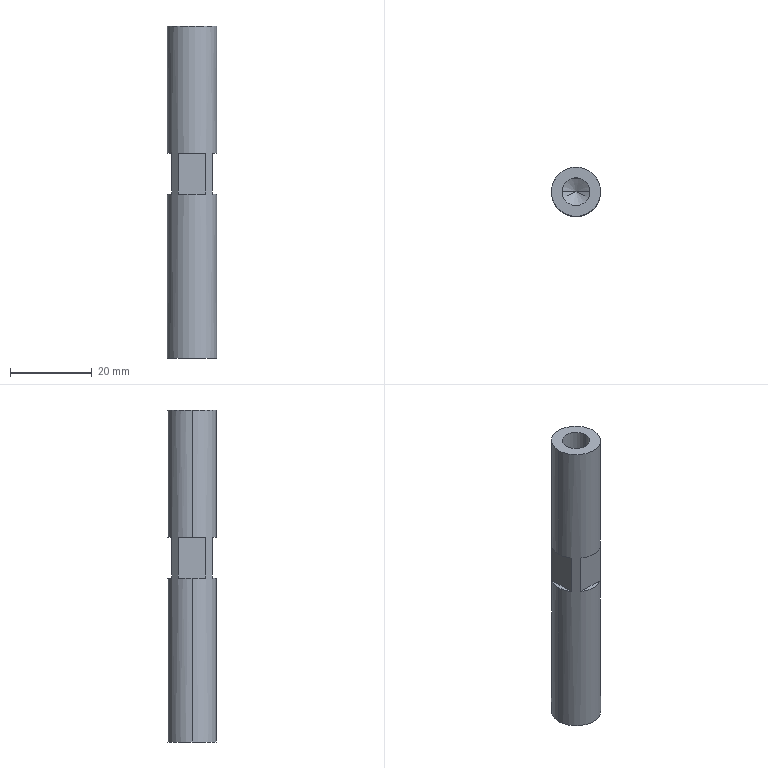Part | STEP file | 44-02-10 Ear Forming Connecting Rod | 1 solid | 24 faces | box 12 x 12 x 81 mm | volume 7569 mm3 | plane 14 | cylinder 6 | cone 4 | commonest cylinder face diameters 6.8 x4 12 x2
STEP:
#1=CARTESIAN_POINT('',(0.,0.,0.));
#2=DIRECTION('',(0.,0.,1.));
#3=DIRECTION('',(1.,0.,0.));
#4=AXIS2_PLACEMENT_3D('',#1,#2,#3);
#5=CARTESIAN_POINT('',(-3.4,0.,-21.75));
#6=VERTEX_POINT('',#5);
#7=CARTESIAN_POINT('',(-3.4,0.,-40.5));
#8=VERTEX_POINT('',#7);
#9=CARTESIAN_POINT('',(-3.4,0.,-40.5));
#10=DIRECTION('',(0.,0.,-1.));
#11=VECTOR('',#10,1.);
#12=LINE('',#9,#11);
#13=CARTESIAN_POINT('',(0.,0.,-40.5));
#14=DIRECTION('',(0.,0.,-1.));
#15=DIRECTION('',(-1.,0.,0.));
#16=AXIS2_PLACEMENT_3D('',#13,#14,#15);
#17=CYLINDRICAL_SURFACE('',#16,3.4);
#18=CARTESIAN_POINT('',(6.283,0.));
#19=DIRECTION('',(0.,1.));
#20=VECTOR('',#19,1.);
#21=LINE('',#18,#20);
#22=(GEOMETRIC_REPRESENTATION_CONTEXT(2)PARAMETRIC_REPRESENTATION_CONTEXT()REPRESENTATION_CONTEXT('',''));
#23=DEFINITIONAL_REPRESENTATION('',(#21),#22);
#24=PCURVE('',#17,#23);
#25=CARTESIAN_POINT('',(0.,0.,-40.5));
#26=DIRECTION('',(0.,0.,-1.));
#27=DIRECTION('',(-1.,0.,0.));
#28=AXIS2_PLACEMENT_3D('',#25,#26,#27);
#29=CYLINDRICAL_SURFACE('',#28,3.4);
#30=CARTESIAN_POINT('',(0.,0.));
#31=DIRECTION('',(0.,1.));
#32=VECTOR('',#31,1.);
#33=LINE('',#30,#32);
#34=(GEOMETRIC_REPRESENTATION_CONTEXT(2)PARAMETRIC_REPRESENTATION_CONTEXT()REPRESENTATION_CONTEXT('',''));
#35=DEFINITIONAL_REPRESENTATION('',(#33),#34);
#36=PCURVE('',#29,#35);
#37=SURFACE_CURVE('',#12,(#24,#36),.PCURVE_S1.);
#38=EDGE_CURVE('',#6,#8,#37,.T.);
#39=ORIENTED_EDGE('',*,*,#38,.T.);
#40=CARTESIAN_POINT('',(3.4,0.,-40.5));
#41=VERTEX_POINT('',#40);
#42=CARTESIAN_POINT('',(0.,0.,-40.5));
#43=DIRECTION('',(0.,0.,-1.));
#44=DIRECTION('',(-1.,0.,0.));
#45=AXIS2_PLACEMENT_3D('',#42,#43,#44);
#46=CIRCLE('',#45,3.4);
#47=CARTESIAN_POINT('',(0.,0.));
#48=DIRECTION('',(1.,0.));
#49=VECTOR('',#48,1.);
#50=LINE('',#47,#49);
#51=(GEOMETRIC_REPRESENTATION_CONTEXT(2)PARAMETRIC_REPRESENTATION_CONTEXT()REPRESENTATION_CONTEXT('',''));
#52=DEFINITIONAL_REPRESENTATION('',(#50),#51);
#53=PCURVE('',#17,#52);
#54=CARTESIAN_POINT('',(0.,0.,-40.5));
#55=DIRECTION('',(0.,0.,1.));
#56=DIRECTION('',(1.,0.,0.));
#57=AXIS2_PLACEMENT_3D('',#54,#55,#56);
#58=PLANE('',#57);
#59=CARTESIAN_POINT('',(-3.4,0.));
#60=CARTESIAN_POINT('',(-3.4,5.889));
#61=CARTESIAN_POINT('',(1.7,2.944));
#62=CARTESIAN_POINT('',(6.8,0.));
#63=CARTESIAN_POINT('',(1.7,-2.944));
#64=CARTESIAN_POINT('',(-3.4,-5.889));
#65=CARTESIAN_POINT('',(-3.4,0.));
#66=(BOUNDED_CURVE()B_SPLINE_CURVE(2,(#59,#60,#61,#62,#63,#64,#65),.UNSPECIFIED.,.T.,.F.)B_SPLINE_CURVE_WITH_KNOTS((1,2,2,2,2,1),(-2.094,0.,2.094,4.189,6.283,8.378),.UNSPECIFIED.)CURVE()GEOMETRIC_REPRESENTATION_ITEM()RATIONAL_B_SPLINE_CURVE((1.,0.5,1.,0.5,1.,0.5,1.))REPRESENTATION_ITEM(''));
#67=(GEOMETRIC_REPRESENTATION_CONTEXT(2)PARAMETRIC_REPRESENTATION_CONTEXT()REPRESENTATION_CONTEXT('',''));
#68=DEFINITIONAL_REPRESENTATION('',(#66),#67);
#69=PCURVE('',#58,#68);
#70=SURFACE_CURVE('',#46,(#53,#69),.PCURVE_S1.);
#71=EDGE_CURVE('',#41,#8,#70,.T.);
#72=ORIENTED_EDGE('',*,*,#71,.F.);
#73=CARTESIAN_POINT('',(3.4,0.,-21.75));
#74=VERTEX_POINT('',#73);
#75=CARTESIAN_POINT('',(3.4,0.,-40.5));
#76=DIRECTION('',(0.,0.,-1.));
#77=VECTOR('',#76,1.);
#78=LINE('',#75,#77);
#79=CARTESIAN_POINT('',(3.142,0.));
#80=DIRECTION('',(0.,1.));
#81=VECTOR('',#80,1.);
#82=LINE('',#79,#81);
#83=(GEOMETRIC_REPRESENTATION_CONTEXT(2)PARAMETRIC_REPRESENTATION_CONTEXT()REPRESENTATION_CONTEXT('',''));
#84=DEFINITIONAL_REPRESENTATION('',(#82),#83);
#85=PCURVE('',#17,#84);
#86=CARTESIAN_POINT('',(3.142,0.));
#87=DIRECTION('',(0.,1.));
#88=VECTOR('',#87,1.);
#89=LINE('',#86,#88);
#90=(GEOMETRIC_REPRESENTATION_CONTEXT(2)PARAMETRIC_REPRESENTATION_CONTEXT()REPRESENTATION_CONTEXT('',''));
#91=DEFINITIONAL_REPRESENTATION('',(#89),#90);
#92=PCURVE('',#29,#91);
#93=SURFACE_CURVE('',#78,(#85,#92),.PCURVE_S1.);
#94=EDGE_CURVE('',#74,#41,#93,.T.);
#95=ORIENTED_EDGE('',*,*,#94,.F.);
#96=CARTESIAN_POINT('',(0.,0.,-21.75));
#97=DIRECTION('',(0.,0.,-1.));
#98=DIRECTION('',(-1.,0.,0.));
#99=AXIS2_PLACEMENT_3D('',#96,#97,#98);
#100=CIRCLE('',#99,3.4);
#101=CARTESIAN_POINT('',(0.,-18.75));
#102=DIRECTION('',(1.,0.));
#103=VECTOR('',#102,1.);
#104=LINE('',#101,#103);
#105=(GEOMETRIC_REPRESENTATION_CONTEXT(2)PARAMETRIC_REPRESENTATION_CONTEXT()REPRESENTATION_CONTEXT('',''));
#106=DEFINITIONAL_REPRESENTATION('',(#104),#105);
#107=PCURVE('',#17,#106);
#108=CARTESIAN_POINT('',(0.,0.,-21.75));
#109=DIRECTION('',(0.,0.,-1.));
#110=DIRECTION('',(-1.,0.,0.));
#111=AXIS2_PLACEMENT_3D('',#108,#109,#110);
#112=CONICAL_SURFACE('',#111,3.4,1.03);
#113=CARTESIAN_POINT('',(0.,0.));
#114=DIRECTION('',(1.,0.));
#115=VECTOR('',#114,1.);
#116=LINE('',#113,#115);
#117=(GEOMETRIC_REPRESENTATION_CONTEXT(2)PARAMETRIC_REPRESENTATION_CONTEXT()REPRESENTATION_CONTEXT('',''));
#118=DEFINITIONAL_REPRESENTATION('',(#116),#117);
#119=PCURVE('',#112,#118);
#120=SURFACE_CURVE('',#100,(#107,#119),.PCURVE_S1.);
#121=EDGE_CURVE('',#74,#6,#120,.T.);
#122=ORIENTED_EDGE('',*,*,#121,.T.);
#123=EDGE_LOOP('',(#39,#72,#95,#122));
#124=FACE_BOUND('',#123,.F.);
#125=ADVANCED_FACE('',(#124),#17,.F.);
#126=ORIENTED_EDGE('',*,*,#121,.F.);
#127=CARTESIAN_POINT('',(0.,0.,-19.707));
#128=VERTEX_POINT('',#127);
#129=CARTESIAN_POINT('',(3.4,0.,-21.75));
#130=DIRECTION('',(0.8572,0.,-0.515));
#131=VECTOR('',#130,1.);
#132=LINE('',#129,#131);
#133=CARTESIAN_POINT('',(3.142,0.));
#134=DIRECTION('',(0.,1.));
#135=VECTOR('',#134,1.);
#136=LINE('',#133,#135);
#137=(GEOMETRIC_REPRESENTATION_CONTEXT(2)PARAMETRIC_REPRESENTATION_CONTEXT()REPRESENTATION_CONTEXT('',''));
#138=DEFINITIONAL_REPRESENTATION('',(#136),#137);
#139=PCURVE('',#112,#138);
#140=CARTESIAN_POINT('',(0.,0.,-21.75));
#141=DIRECTION('',(0.,0.,-1.));
#142=DIRECTION('',(-1.,0.,0.));
#143=AXIS2_PLACEMENT_3D('',#140,#141,#142);
#144=CONICAL_SURFACE('',#143,3.4,1.03);
#145=CARTESIAN_POINT('',(3.142,0.));
#146=DIRECTION('',(0.,1.));
#147=VECTOR('',#146,1.);
#148=LINE('',#145,#147);
#149=(GEOMETRIC_REPRESENTATION_CONTEXT(2)PARAMETRIC_REPRESENTATION_CONTEXT()REPRESENTATION_CONTEXT('',''));
#150=DEFINITIONAL_REPRESENTATION('',(#148),#149);
#151=PCURVE('',#144,#150);
#152=SURFACE_CURVE('',#132,(#139,#151),.PCURVE_S1.);
#153=EDGE_CURVE('',#128,#74,#152,.T.);
#154=ORIENTED_EDGE('',*,*,#153,.F.);
#155=CARTESIAN_POINT('',(-3.4,0.,-21.75));
#156=DIRECTION('',(-0.8572,0.,-0.515));
#157=VECTOR('',#156,1.);
#158=LINE('',#155,#157);
#159=CARTESIAN_POINT('',(6.283,0.));
#160=DIRECTION('',(0.,1.));
#161=VECTOR('',#160,1.);
#162=LINE('',#159,#161);
#163=(GEOMETRIC_REPRESENTATION_CONTEXT(2)PARAMETRIC_REPRESENTATION_CONTEXT()REPRESENTATION_CONTEXT('',''));
#164=DEFINITIONAL_REPRESENTATION('',(#162),#163);
#165=PCURVE('',#112,#164);
#166=CARTESIAN_POINT('',(0.,0.));
#167=DIRECTION('',(0.,1.));
#168=VECTOR('',#167,1.);
#169=LINE('',#166,#168);
#170=(GEOMETRIC_REPRESENTATION_CONTEXT(2)PARAMETRIC_REPRESENTATION_CONTEXT()REPRESENTATION_CONTEXT('',''));
#171=DEFINITIONAL_REPRESENTATION('',(#169),#170);
#172=PCURVE('',#144,#171);
#173=SURFACE_CURVE('',#158,(#165,#172),.PCURVE_S1.);
#174=EDGE_CURVE('',#128,#6,#173,.T.);
#175=ORIENTED_EDGE('',*,*,#174,.T.);
#176=EDGE_LOOP('',(#126,#154,#175));
#177=FACE_BOUND('',#176,.F.);
#178=ADVANCED_FACE('',(#177),#112,.F.);
#179=CARTESIAN_POINT('',(3.4,0.,21.75));
#180=VERTEX_POINT('',#179);
#181=CARTESIAN_POINT('',(3.4,0.,40.5));
#182=VERTEX_POINT('',#181);
#183=CARTESIAN_POINT('',(3.4,0.,40.5));
#184=DIRECTION('',(0.,0.,1.));
#185=VECTOR('',#184,1.);
#186=LINE('',#183,#185);
#187=CARTESIAN_POINT('',(0.,0.,40.5));
#188=DIRECTION('',(0.,0.,1.));
#189=DIRECTION('',(1.,0.,0.));
#190=AXIS2_PLACEMENT_3D('',#187,#188,#189);
#191=CYLINDRICAL_SURFACE('',#190,3.4);
#192=CARTESIAN_POINT('',(6.283,0.));
#193=DIRECTION('',(0.,1.));
#194=VECTOR('',#193,1.);
#195=LINE('',#192,#194);
#196=(GEOMETRIC_REPRESENTATION_CONTEXT(2)PARAMETRIC_REPRESENTATION_CONTEXT()REPRESENTATION_CONTEXT('',''));
#197=DEFINITIONAL_REPRESENTATION('',(#195),#196);
#198=PCURVE('',#191,#197);
#199=CARTESIAN_POINT('',(0.,0.,40.5));
#200=DIRECTION('',(0.,0.,1.));
#201=DIRECTION('',(1.,0.,0.));
#202=AXIS2_PLACEMENT_3D('',#199,#200,#201);
#203=CYLINDRICAL_SURFACE('',#202,3.4);
#204=CARTESIAN_POINT('',(0.,0.));
#205=DIRECTION('',(0.,1.));
#206=VECTOR('',#205,1.);
#207=LINE('',#204,#206);
#208=(GEOMETRIC_REPRESENTATION_CONTEXT(2)PARAMETRIC_REPRESENTATION_CONTEXT()REPRESENTATION_CONTEXT('',''));
#209=DEFINITIONAL_REPRESENTATION('',(#207),#208);
#210=PCURVE('',#203,#209);
#211=SURFACE_CURVE('',#186,(#198,#210),.PCURVE_S1.);
#212=EDGE_CURVE('',#180,#182,#211,.T.);
#213=ORIENTED_EDGE('',*,*,#212,.T.);
#214=CARTESIAN_POINT('',(-3.4,0.,40.5));
#215=VERTEX_POINT('',#214);
#216=CARTESIAN_POINT('',(0.,0.,40.5));
#217=DIRECTION('',(0.,0.,1.));
#218=DIRECTION('',(1.,0.,0.));
#219=AXIS2_PLACEMENT_3D('',#216,#217,#218);
#220=CIRCLE('',#219,3.4);
#221=CARTESIAN_POINT('',(0.,0.));
#222=DIRECTION('',(1.,0.));
#223=VECTOR('',#222,1.);
#224=LINE('',#221,#223);
#225=(GEOMETRIC_REPRESENTATION_CONTEXT(2)PARAMETRIC_REPRESENTATION_CONTEXT()REPRESENTATION_CONTEXT('',''));
#226=DEFINITIONAL_REPRESENTATION('',(#224),#225);
#227=PCURVE('',#191,#226);
#228=CARTESIAN_POINT('',(0.,0.,40.5));
#229=DIRECTION('',(0.,0.,1.));
#230=DIRECTION('',(1.,0.,0.));
#231=AXIS2_PLACEMENT_3D('',#228,#229,#230);
#232=PLANE('',#231);
#233=CARTESIAN_POINT('',(0.,0.));
#234=DIRECTION('',(1.,0.));
#235=AXIS2_PLACEMENT_2D('',#233,#234);
#236=CIRCLE('',#235,3.4);
#237=(GEOMETRIC_REPRESENTATION_CONTEXT(2)PARAMETRIC_REPRESENTATION_CONTEXT()REPRESENTATION_CONTEXT('',''));
#238=DEFINITIONAL_REPRESENTATION('',(#236),#237);
#239=PCURVE('',#232,#238);
#240=SURFACE_CURVE('',#220,(#227,#239),.PCURVE_S1.);
#241=EDGE_CURVE('',#215,#182,#240,.T.);
#242=ORIENTED_EDGE('',*,*,#241,.F.);
#243=CARTESIAN_POINT('',(-3.4,0.,21.75));
#244=VERTEX_POINT('',#243);
#245=CARTESIAN_POINT('',(-3.4,0.,40.5));
#246=DIRECTION('',(0.,0.,1.));
#247=VECTOR('',#246,1.);
#248=LINE('',#245,#247);
#249=CARTESIAN_POINT('',(3.142,0.));
#250=DIRECTION('',(0.,1.));
#251=VECTOR('',#250,1.);
#252=LINE('',#249,#251);
#253=(GEOMETRIC_REPRESENTATION_CONTEXT(2)PARAMETRIC_REPRESENTATION_CONTEXT()REPRESENTATION_CONTEXT('',''));
#254=DEFINITIONAL_REPRESENTATION('',(#252),#253);
#255=PCURVE('',#191,#254);
#256=CARTESIAN_POINT('',(3.142,0.));
#257=DIRECTION('',(0.,1.));
#258=VECTOR('',#257,1.);
#259=LINE('',#256,#258);
#260=(GEOMETRIC_REPRESENTATION_CONTEXT(2)PARAMETRIC_REPRESENTATION_CONTEXT()REPRESENTATION_CONTEXT('',''));
#261=DEFINITIONAL_REPRESENTATION('',(#259),#260);
#262=PCURVE('',#203,#261);
#263=SURFACE_CURVE('',#248,(#255,#262),.PCURVE_S1.);
#264=EDGE_CURVE('',#244,#215,#263,.T.);
#265=ORIENTED_EDGE('',*,*,#264,.F.);
#266=CARTESIAN_POINT('',(0.,0.,21.75));
#267=DIRECTION('',(0.,0.,1.));
#268=DIRECTION('',(1.,0.,0.));
#269=AXIS2_PLACEMENT_3D('',#266,#267,#268);
#270=CIRCLE('',#269,3.4);
#271=CARTESIAN_POINT('',(0.,-18.75));
#272=DIRECTION('',(1.,0.));
#273=VECTOR('',#272,1.);
#274=LINE('',#271,#273);
#275=(GEOMETRIC_REPRESENTATION_CONTEXT(2)PARAMETRIC_REPRESENTATION_CONTEXT()REPRESENTATION_CONTEXT('',''));
#276=DEFINITIONAL_REPRESENTATION('',(#274),#275);
#277=PCURVE('',#191,#276);
#278=CARTESIAN_POINT('',(0.,0.,21.75));
#279=DIRECTION('',(0.,0.,1.));
#280=DIRECTION('',(1.,0.,0.));
#281=AXIS2_PLACEMENT_3D('',#278,#279,#280);
#282=CONICAL_SURFACE('',#281,3.4,1.03);
#283=CARTESIAN_POINT('',(0.,0.));
#284=DIRECTION('',(1.,0.));
#285=VECTOR('',#284,1.);
#286=LINE('',#283,#285);
#287=(GEOMETRIC_REPRESENTATION_CONTEXT(2)PARAMETRIC_REPRESENTATION_CONTEXT()REPRESENTATION_CONTEXT('',''));
#288=DEFINITIONAL_REPRESENTATION('',(#286),#287);
#289=PCURVE('',#282,#288);
#290=SURFACE_CURVE('',#270,(#277,#289),.PCURVE_S1.);
#291=EDGE_CURVE('',#244,#180,#290,.T.);
#292=ORIENTED_EDGE('',*,*,#291,.T.);
#293=EDGE_LOOP('',(#213,#242,#265,#292));
#294=FACE_BOUND('',#293,.F.);
#295=ADVANCED_FACE('',(#294),#191,.F.);
#296=ORIENTED_EDGE('',*,*,#291,.F.);
#297=CARTESIAN_POINT('',(0.,0.,19.707));
#298=VERTEX_POINT('',#297);
#299=CARTESIAN_POINT('',(-3.4,0.,21.75));
#300=DIRECTION('',(-0.8572,0.,0.515));
#301=VECTOR('',#300,1.);
#302=LINE('',#299,#301);
#303=CARTESIAN_POINT('',(3.142,0.));
#304=DIRECTION('',(0.,1.));
#305=VECTOR('',#304,1.);
#306=LINE('',#303,#305);
#307=(GEOMETRIC_REPRESENTATION_CONTEXT(2)PARAMETRIC_REPRESENTATION_CONTEXT()REPRESENTATION_CONTEXT('',''));
#308=DEFINITIONAL_REPRESENTATION('',(#306),#307);
#309=PCURVE('',#282,#308);
#310=CARTESIAN_POINT('',(0.,0.,21.75));
#311=DIRECTION('',(0.,0.,1.));
#312=DIRECTION('',(1.,0.,0.));
#313=AXIS2_PLACEMENT_3D('',#310,#311,#312);
#314=CONICAL_SURFACE('',#313,3.4,1.03);
#315=CARTESIAN_POINT('',(3.142,0.));
#316=DIRECTION('',(0.,1.));
#317=VECTOR('',#316,1.);
#318=LINE('',#315,#317);
#319=(GEOMETRIC_REPRESENTATION_CONTEXT(2)PARAMETRIC_REPRESENTATION_CONTEXT()REPRESENTATION_CONTEXT('',''));
#320=DEFINITIONAL_REPRESENTATION('',(#318),#319);
#321=PCURVE('',#314,#320);
#322=SURFACE_CURVE('',#302,(#309,#321),.PCURVE_S1.);
#323=EDGE_CURVE('',#298,#244,#322,.T.);
#324=ORIENTED_EDGE('',*,*,#323,.F.);
#325=CARTESIAN_POINT('',(3.4,0.,21.75));
#326=DIRECTION('',(0.8572,0.,0.515));
#327=VECTOR('',#326,1.);
#328=LINE('',#325,#327);
#329=CARTESIAN_POINT('',(6.283,0.));
#330=DIRECTION('',(0.,1.));
#331=VECTOR('',#330,1.);
#332=LINE('',#329,#331);
#333=(GEOMETRIC_REPRESENTATION_CONTEXT(2)PARAMETRIC_REPRESENTATION_CONTEXT()REPRESENTATION_CONTEXT('',''));
#334=DEFINITIONAL_REPRESENTATION('',(#332),#333);
#335=PCURVE('',#282,#334);
#336=CARTESIAN_POINT('',(0.,0.));
#337=DIRECTION('',(0.,1.));
#338=VECTOR('',#337,1.);
#339=LINE('',#336,#338);
#340=(GEOMETRIC_REPRESENTATION_CONTEXT(2)PARAMETRIC_REPRESENTATION_CONTEXT()REPRESENTATION_CONTEXT('',''));
#341=DEFINITIONAL_REPRESENTATION('',(#339),#340);
#342=PCURVE('',#314,#341);
#343=SURFACE_CURVE('',#328,(#335,#342),.PCURVE_S1.);
#344=EDGE_CURVE('',#298,#180,#343,.T.);
#345=ORIENTED_EDGE('',*,*,#344,.T.);
#346=EDGE_LOOP('',(#296,#324,#345));
#347=FACE_BOUND('',#346,.F.);
#348=ADVANCED_FACE('',(#347),#282,.F.);
#349=CARTESIAN_POINT('',(3.317,5.,9.5));
#350=VERTEX_POINT('',#349);
#351=CARTESIAN_POINT('',(-3.317,5.,9.5));
#352=VERTEX_POINT('',#351);
#353=CARTESIAN_POINT('',(0.,0.,9.5));
#354=DIRECTION('',(0.,0.,1.));
#355=DIRECTION('',(1.,0.,0.));
#356=AXIS2_PLACEMENT_3D('',#353,#354,#355);
#357=CIRCLE('',#356,6.);
#358=CARTESIAN_POINT('',(0.,0.,40.5));
#359=DIRECTION('',(0.,0.,-1.));
#360=DIRECTION('',(-1.,0.,0.));
#361=AXIS2_PLACEMENT_3D('',#358,#359,#360);
#362=CYLINDRICAL_SURFACE('',#361,6.);
#363=CARTESIAN_POINT('',(3.142,31.));
#364=DIRECTION('',(-1.,0.));
#365=VECTOR('',#364,1.);
#366=LINE('',#363,#365);
#367=(GEOMETRIC_REPRESENTATION_CONTEXT(2)PARAMETRIC_REPRESENTATION_CONTEXT()REPRESENTATION_CONTEXT('',''));
#368=DEFINITIONAL_REPRESENTATION('',(#366),#367);
#369=PCURVE('',#362,#368);
#370=CARTESIAN_POINT('',(-10.,11.671,9.5));
#371=DIRECTION('',(0.,0.,1.));
#372=DIRECTION('',(1.,0.,0.));
#373=AXIS2_PLACEMENT_3D('',#370,#371,#372);
#374=PLANE('',#373);
#375=CARTESIAN_POINT('',(10.,-11.671));
#376=DIRECTION('',(1.,0.));
#377=AXIS2_PLACEMENT_2D('',#375,#376);
#378=CIRCLE('',#377,6.);
#379=(GEOMETRIC_REPRESENTATION_CONTEXT(2)PARAMETRIC_REPRESENTATION_CONTEXT()REPRESENTATION_CONTEXT('',''));
#380=DEFINITIONAL_REPRESENTATION('',(#378),#379);
#381=PCURVE('',#374,#380);
#382=SURFACE_CURVE('',#357,(#369,#381),.PCURVE_S1.);
#383=EDGE_CURVE('',#350,#352,#382,.T.);
#384=ORIENTED_EDGE('',*,*,#383,.T.);
#385=CARTESIAN_POINT('',(-3.317,5.,-0.5));
#386=VERTEX_POINT('',#385);
#387=CARTESIAN_POINT('',(-3.317,5.,40.5));
#388=DIRECTION('',(0.,0.,-1.));
#389=VECTOR('',#388,1.);
#390=LINE('',#387,#389);
#391=CARTESIAN_POINT('',(0.9851,0.));
#392=DIRECTION('',(0.,1.));
#393=VECTOR('',#392,1.);
#394=LINE('',#391,#393);
#395=(GEOMETRIC_REPRESENTATION_CONTEXT(2)PARAMETRIC_REPRESENTATION_CONTEXT()REPRESENTATION_CONTEXT('',''));
#396=DEFINITIONAL_REPRESENTATION('',(#394),#395);
#397=PCURVE('',#362,#396);
#398=CARTESIAN_POINT('',(-10.,5.,9.5));
#399=DIRECTION('',(0.,-1.,0.));
#400=DIRECTION('',(0.,0.,-1.));
#401=AXIS2_PLACEMENT_3D('',#398,#399,#400);
#402=PLANE('',#401);
#403=CARTESIAN_POINT('',(-31.,6.683));
#404=DIRECTION('',(1.,0.));
#405=VECTOR('',#404,1.);
#406=LINE('',#403,#405);
#407=(GEOMETRIC_REPRESENTATION_CONTEXT(2)PARAMETRIC_REPRESENTATION_CONTEXT()REPRESENTATION_CONTEXT('',''));
#408=DEFINITIONAL_REPRESENTATION('',(#406),#407);
#409=PCURVE('',#402,#408);
#410=SURFACE_CURVE('',#390,(#397,#409),.PCURVE_S1.);
#411=EDGE_CURVE('',#352,#386,#410,.T.);
#412=ORIENTED_EDGE('',*,*,#411,.T.);
#413=CARTESIAN_POINT('',(3.317,5.,-0.5));
#414=VERTEX_POINT('',#413);
#415=CARTESIAN_POINT('',(0.,0.,-0.5));
#416=DIRECTION('',(0.,0.,-1.));
#417=DIRECTION('',(0.,1.,0.));
#418=AXIS2_PLACEMENT_3D('',#415,#416,#417);
#419=CIRCLE('',#418,6.);
#420=CARTESIAN_POINT('',(-4.712,41.));
#421=DIRECTION('',(1.,0.));
#422=VECTOR('',#421,1.);
#423=LINE('',#420,#422);
#424=(GEOMETRIC_REPRESENTATION_CONTEXT(2)PARAMETRIC_REPRESENTATION_CONTEXT()REPRESENTATION_CONTEXT('',''));
#425=DEFINITIONAL_REPRESENTATION('',(#423),#424);
#426=PCURVE('',#362,#425);
#427=CARTESIAN_POINT('',(-10.,11.671,-0.5));
#428=DIRECTION('',(0.,0.,-1.));
#429=DIRECTION('',(0.,1.,0.));
#430=AXIS2_PLACEMENT_3D('',#427,#428,#429);
#431=PLANE('',#430);
#432=CARTESIAN_POINT('',(-11.671,10.));
#433=DIRECTION('',(1.,0.));
#434=AXIS2_PLACEMENT_2D('',#432,#433);
#435=CIRCLE('',#434,6.);
#436=(GEOMETRIC_REPRESENTATION_CONTEXT(2)PARAMETRIC_REPRESENTATION_CONTEXT()REPRESENTATION_CONTEXT('',''));
#437=DEFINITIONAL_REPRESENTATION('',(#435),#436);
#438=PCURVE('',#431,#437);
#439=SURFACE_CURVE('',#419,(#426,#438),.PCURVE_S1.);
#440=EDGE_CURVE('',#386,#414,#439,.T.);
#441=ORIENTED_EDGE('',*,*,#440,.T.);
#442=CARTESIAN_POINT('',(3.317,5.,40.5));
#443=DIRECTION('',(0.,0.,1.));
#444=VECTOR('',#443,1.);
#445=LINE('',#442,#444);
#446=CARTESIAN_POINT('',(2.156,0.));
#447=DIRECTION('',(0.,-1.));
#448=VECTOR('',#447,1.);
#449=LINE('',#446,#448);
#450=(GEOMETRIC_REPRESENTATION_CONTEXT(2)PARAMETRIC_REPRESENTATION_CONTEXT()REPRESENTATION_CONTEXT('',''));
#451=DEFINITIONAL_REPRESENTATION('',(#449),#450);
#452=PCURVE('',#362,#451);
#453=CARTESIAN_POINT('',(-31.,13.317));
#454=DIRECTION('',(-1.,0.));
#455=VECTOR('',#454,1.);
#456=LINE('',#453,#455);
#457=(GEOMETRIC_REPRESENTATION_CONTEXT(2)PARAMETRIC_REPRESENTATION_CONTEXT()REPRESENTATION_CONTEXT('',''));
#458=DEFINITIONAL_REPRESENTATION('',(#456),#457);
#459=PCURVE('',#402,#458);
#460=SURFACE_CURVE('',#445,(#452,#459),.PCURVE_S1.);
#461=EDGE_CURVE('',#414,#350,#460,.T.);
#462=ORIENTED_EDGE('',*,*,#461,.T.);
#463=EDGE_LOOP('',(#384,#412,#441,#462));
#464=FACE_BOUND('',#463,.T.);
#465=CARTESIAN_POINT('',(6.,0.,40.5));
#466=VERTEX_POINT('',#465);
#467=CARTESIAN_POINT('',(-6.,0.,40.5));
#468=VERTEX_POINT('',#467);
#469=CARTESIAN_POINT('',(0.,0.,40.5));
#470=DIRECTION('',(0.,0.,1.));
#471=DIRECTION('',(1.,0.,0.));
#472=AXIS2_PLACEMENT_3D('',#469,#470,#471);
#473=CIRCLE('',#472,6.);
#474=CARTESIAN_POINT('',(3.142,0.));
#475=DIRECTION('',(-1.,0.));
#476=VECTOR('',#475,1.);
#477=LINE('',#474,#476);
#478=(GEOMETRIC_REPRESENTATION_CONTEXT(2)PARAMETRIC_REPRESENTATION_CONTEXT()REPRESENTATION_CONTEXT('',''));
#479=DEFINITIONAL_REPRESENTATION('',(#477),#478);
#480=PCURVE('',#362,#479);
#481=CARTESIAN_POINT('',(0.,0.));
#482=DIRECTION('',(1.,0.));
#483=AXIS2_PLACEMENT_2D('',#481,#482);
#484=CIRCLE('',#483,6.);
#485=(GEOMETRIC_REPRESENTATION_CONTEXT(2)PARAMETRIC_REPRESENTATION_CONTEXT()REPRESENTATION_CONTEXT('',''));
#486=DEFINITIONAL_REPRESENTATION('',(#484),#485);
#487=PCURVE('',#232,#486);
#488=SURFACE_CURVE('',#473,(#480,#487),.PCURVE_S1.);
#489=EDGE_CURVE('',#466,#468,#488,.T.);
#490=ORIENTED_EDGE('',*,*,#489,.F.);
#491=CARTESIAN_POINT('',(6.,0.,9.5));
#492=VERTEX_POINT('',#491);
#493=CARTESIAN_POINT('',(6.,0.,40.5));
#494=DIRECTION('',(0.,0.,-1.));
#495=VECTOR('',#494,1.);
#496=LINE('',#493,#495);
#497=CARTESIAN_POINT('',(3.142,0.));
#498=DIRECTION('',(0.,1.));
#499=VECTOR('',#498,1.);
#500=LINE('',#497,#499);
#501=(GEOMETRIC_REPRESENTATION_CONTEXT(2)PARAMETRIC_REPRESENTATION_CONTEXT()REPRESENTATION_CONTEXT('',''));
#502=DEFINITIONAL_REPRESENTATION('',(#500),#501);
#503=PCURVE('',#362,#502);
#504=CARTESIAN_POINT('',(0.,0.,40.5));
#505=DIRECTION('',(0.,0.,-1.));
#506=DIRECTION('',(-1.,0.,0.));
#507=AXIS2_PLACEMENT_3D('',#504,#505,#506);
#508=CYLINDRICAL_SURFACE('',#507,6.);
#509=CARTESIAN_POINT('',(3.142,0.));
#510=DIRECTION('',(0.,1.));
#511=VECTOR('',#510,1.);
#512=LINE('',#509,#511);
#513=(GEOMETRIC_REPRESENTATION_CONTEXT(2)PARAMETRIC_REPRESENTATION_CONTEXT()REPRESENTATION_CONTEXT('',''));
#514=DEFINITIONAL_REPRESENTATION('',(#512),#513);
#515=PCURVE('',#508,#514);
#516=SURFACE_CURVE('',#496,(#503,#515),.PCURVE_S1.);
#517=EDGE_CURVE('',#466,#492,#516,.T.);
#518=ORIENTED_EDGE('',*,*,#517,.T.);
#519=CARTESIAN_POINT('',(5.,3.317,9.5));
#520=VERTEX_POINT('',#519);
#521=CARTESIAN_POINT('',(0.,0.,9.5));
#522=DIRECTION('',(0.,0.,-1.));
#523=DIRECTION('',(-1.,0.,0.));
#524=AXIS2_PLACEMENT_3D('',#521,#522,#523);
#525=CIRCLE('',#524,6.);
#526=CARTESIAN_POINT('',(0.,31.));
#527=DIRECTION('',(1.,0.));
#528=VECTOR('',#527,1.);
#529=LINE('',#526,#528);
#530=(GEOMETRIC_REPRESENTATION_CONTEXT(2)PARAMETRIC_REPRESENTATION_CONTEXT()REPRESENTATION_CONTEXT('',''));
#531=DEFINITIONAL_REPRESENTATION('',(#529),#530);
#532=PCURVE('',#362,#531);
#533=CARTESIAN_POINT('',(13.922,-10.,9.5));
#534=DIRECTION('',(0.,0.,-1.));
#535=DIRECTION('',(-1.,0.,0.));
#536=AXIS2_PLACEMENT_3D('',#533,#534,#535);
#537=PLANE('',#536);
#538=CARTESIAN_POINT('',(13.922,10.));
#539=DIRECTION('',(1.,0.));
#540=AXIS2_PLACEMENT_2D('',#538,#539);
#541=CIRCLE('',#540,6.);
#542=(GEOMETRIC_REPRESENTATION_CONTEXT(2)PARAMETRIC_REPRESENTATION_CONTEXT()REPRESENTATION_CONTEXT('',''));
#543=DEFINITIONAL_REPRESENTATION('',(#541),#542);
#544=PCURVE('',#537,#543);
#545=SURFACE_CURVE('',#525,(#532,#544),.PCURVE_S1.);
#546=EDGE_CURVE('',#520,#492,#545,.T.);
#547=ORIENTED_EDGE('',*,*,#546,.F.);
#548=CARTESIAN_POINT('',(5.,3.317,-0.5));
#549=VERTEX_POINT('',#548);
#550=CARTESIAN_POINT('',(5.,3.317,40.5));
#551=DIRECTION('',(0.,0.,1.));
#552=VECTOR('',#551,1.);
#553=LINE('',#550,#552);
#554=CARTESIAN_POINT('',(2.556,0.));
#555=DIRECTION('',(0.,-1.));
#556=VECTOR('',#555,1.);
#557=LINE('',#554,#556);
#558=(GEOMETRIC_REPRESENTATION_CONTEXT(2)PARAMETRIC_REPRESENTATION_CONTEXT()REPRESENTATION_CONTEXT('',''));
#559=DEFINITIONAL_REPRESENTATION('',(#557),#558);
#560=PCURVE('',#362,#559);
#561=CARTESIAN_POINT('',(5.,-10.,-0.5));
#562=DIRECTION('',(1.,0.,0.));
#563=DIRECTION('',(0.,0.,-1.));
#564=AXIS2_PLACEMENT_3D('',#561,#562,#563);
#565=PLANE('',#564);
#566=CARTESIAN_POINT('',(-41.,13.317));
#567=DIRECTION('',(-1.,0.));
#568=VECTOR('',#567,1.);
#569=LINE('',#566,#568);
#570=(GEOMETRIC_REPRESENTATION_CONTEXT(2)PARAMETRIC_REPRESENTATION_CONTEXT()REPRESENTATION_CONTEXT('',''));
#571=DEFINITIONAL_REPRESENTATION('',(#569),#570);
#572=PCURVE('',#565,#571);
#573=SURFACE_CURVE('',#553,(#560,#572),.PCURVE_S1.);
#574=EDGE_CURVE('',#549,#520,#573,.T.);
#575=ORIENTED_EDGE('',*,*,#574,.F.);
#576=CARTESIAN_POINT('',(6.,0.,-0.5));
#577=VERTEX_POINT('',#576);
#578=CARTESIAN_POINT('',(0.,0.,-0.5));
#579=DIRECTION('',(0.,0.,1.));
#580=DIRECTION('',(1.,0.,0.));
#581=AXIS2_PLACEMENT_3D('',#578,#579,#580);
#582=CIRCLE('',#581,6.);
#583=CARTESIAN_POINT('',(3.142,41.));
#584=DIRECTION('',(-1.,0.));
#585=VECTOR('',#584,1.);
#586=LINE('',#583,#585);
#587=(GEOMETRIC_REPRESENTATION_CONTEXT(2)PARAMETRIC_REPRESENTATION_CONTEXT()REPRESENTATION_CONTEXT('',''));
#588=DEFINITIONAL_REPRESENTATION('',(#586),#587);
#589=PCURVE('',#362,#588);
#590=CARTESIAN_POINT('',(13.922,-10.,-0.5));
#591=DIRECTION('',(0.,0.,1.));
#592=DIRECTION('',(1.,0.,0.));
#593=AXIS2_PLACEMENT_3D('',#590,#591,#592);
#594=PLANE('',#593);
#595=CARTESIAN_POINT('',(-13.922,10.));
#596=DIRECTION('',(1.,0.));
#597=AXIS2_PLACEMENT_2D('',#595,#596);
#598=CIRCLE('',#597,6.);
#599=(GEOMETRIC_REPRESENTATION_CONTEXT(2)PARAMETRIC_REPRESENTATION_CONTEXT()REPRESENTATION_CONTEXT('',''));
#600=DEFINITIONAL_REPRESENTATION('',(#598),#599);
#601=PCURVE('',#594,#600);
#602=SURFACE_CURVE('',#582,(#589,#601),.PCURVE_S1.);
#603=EDGE_CURVE('',#577,#549,#602,.T.);
#604=ORIENTED_EDGE('',*,*,#603,.F.);
#605=CARTESIAN_POINT('',(6.,0.,-40.5));
#606=VERTEX_POINT('',#605);
#607=CARTESIAN_POINT('',(6.,0.,40.5));
#608=DIRECTION('',(0.,0.,-1.));
#609=VECTOR('',#608,1.);
#610=LINE('',#607,#609);
#611=CARTESIAN_POINT('',(3.142,0.));
#612=DIRECTION('',(0.,1.));
#613=VECTOR('',#612,1.);
#614=LINE('',#611,#613);
#615=(GEOMETRIC_REPRESENTATION_CONTEXT(2)PARAMETRIC_REPRESENTATION_CONTEXT()REPRESENTATION_CONTEXT('',''));
#616=DEFINITIONAL_REPRESENTATION('',(#614),#615);
#617=PCURVE('',#362,#616);
#618=CARTESIAN_POINT('',(3.142,0.));
#619=DIRECTION('',(0.,1.));
#620=VECTOR('',#619,1.);
#621=LINE('',#618,#620);
#622=(GEOMETRIC_REPRESENTATION_CONTEXT(2)PARAMETRIC_REPRESENTATION_CONTEXT()REPRESENTATION_CONTEXT('',''));
#623=DEFINITIONAL_REPRESENTATION('',(#621),#622);
#624=PCURVE('',#508,#623);
#625=SURFACE_CURVE('',#610,(#617,#624),.PCURVE_S1.);
#626=EDGE_CURVE('',#577,#606,#625,.T.);
#627=ORIENTED_EDGE('',*,*,#626,.T.);
#628=CARTESIAN_POINT('',(-6.,0.,-40.5));
#629=VERTEX_POINT('',#628);
#630=CARTESIAN_POINT('',(0.,0.,-40.5));
#631=DIRECTION('',(0.,0.,1.));
#632=DIRECTION('',(1.,0.,0.));
#633=AXIS2_PLACEMENT_3D('',#630,#631,#632);
#634=CIRCLE('',#633,6.);
#635=CARTESIAN_POINT('',(3.142,81.));
#636=DIRECTION('',(-1.,0.));
#637=VECTOR('',#636,1.);
#638=LINE('',#635,#637);
#639=(GEOMETRIC_REPRESENTATION_CONTEXT(2)PARAMETRIC_REPRESENTATION_CONTEXT()REPRESENTATION_CONTEXT('',''));
#640=DEFINITIONAL_REPRESENTATION('',(#638),#639);
#641=PCURVE('',#362,#640);
#642=CARTESIAN_POINT('',(0.,0.));
#643=DIRECTION('',(1.,0.));
#644=AXIS2_PLACEMENT_2D('',#642,#643);
#645=CIRCLE('',#644,6.);
#646=(GEOMETRIC_REPRESENTATION_CONTEXT(2)PARAMETRIC_REPRESENTATION_CONTEXT()REPRESENTATION_CONTEXT('',''));
#647=DEFINITIONAL_REPRESENTATION('',(#645),#646);
#648=PCURVE('',#58,#647);
#649=SURFACE_CURVE('',#634,(#641,#648),.PCURVE_S1.);
#650=EDGE_CURVE('',#606,#629,#649,.T.);
#651=ORIENTED_EDGE('',*,*,#650,.T.);
#652=CARTESIAN_POINT('',(-6.,0.,-0.5));
#653=VERTEX_POINT('',#652);
#654=CARTESIAN_POINT('',(-6.,0.,40.5));
#655=DIRECTION('',(0.,0.,-1.));
#656=VECTOR('',#655,1.);
#657=LINE('',#654,#656);
#658=CARTESIAN_POINT('',(0.,0.));
#659=DIRECTION('',(0.,1.));
#660=VECTOR('',#659,1.);
#661=LINE('',#658,#660);
#662=(GEOMETRIC_REPRESENTATION_CONTEXT(2)PARAMETRIC_REPRESENTATION_CONTEXT()REPRESENTATION_CONTEXT('',''));
#663=DEFINITIONAL_REPRESENTATION('',(#661),#662);
#664=PCURVE('',#362,#663);
#665=CARTESIAN_POINT('',(6.283,0.));
#666=DIRECTION('',(0.,1.));
#667=VECTOR('',#666,1.);
#668=LINE('',#665,#667);
#669=(GEOMETRIC_REPRESENTATION_CONTEXT(2)PARAMETRIC_REPRESENTATION_CONTEXT()REPRESENTATION_CONTEXT('',''));
#670=DEFINITIONAL_REPRESENTATION('',(#668),#669);
#671=PCURVE('',#508,#670);
#672=SURFACE_CURVE('',#657,(#664,#671),.PCURVE_S1.);
#673=EDGE_CURVE('',#653,#629,#672,.T.);
#674=ORIENTED_EDGE('',*,*,#673,.F.);
#675=CARTESIAN_POINT('',(-5.,3.317,-0.5));
#676=VERTEX_POINT('',#675);
#677=CARTESIAN_POINT('',(0.,0.,-0.5));
#678=DIRECTION('',(0.,0.,-1.));
#679=DIRECTION('',(-1.,0.,0.));
#680=AXIS2_PLACEMENT_3D('',#677,#678,#679);
#681=CIRCLE('',#680,6.);
#682=CARTESIAN_POINT('',(0.,41.));
#683=DIRECTION('',(1.,0.));
#684=VECTOR('',#683,1.);
#685=LINE('',#682,#684);
#686=(GEOMETRIC_REPRESENTATION_CONTEXT(2)PARAMETRIC_REPRESENTATION_CONTEXT()REPRESENTATION_CONTEXT('',''));
#687=DEFINITIONAL_REPRESENTATION('',(#685),#686);
#688=PCURVE('',#362,#687);
#689=CARTESIAN_POINT('',(-13.922,-10.,-0.5));
#690=DIRECTION('',(0.,0.,-1.));
#691=DIRECTION('',(-1.,0.,0.));
#692=AXIS2_PLACEMENT_3D('',#689,#690,#691);
#693=PLANE('',#692);
#694=CARTESIAN_POINT('',(-13.922,10.));
#695=DIRECTION('',(1.,0.));
#696=AXIS2_PLACEMENT_2D('',#694,#695);
#697=CIRCLE('',#696,6.);
#698=(GEOMETRIC_REPRESENTATION_CONTEXT(2)PARAMETRIC_REPRESENTATION_CONTEXT()REPRESENTATION_CONTEXT('',''));
#699=DEFINITIONAL_REPRESENTATION('',(#697),#698);
#700=PCURVE('',#693,#699);
#701=SURFACE_CURVE('',#681,(#688,#700),.PCURVE_S1.);
#702=EDGE_CURVE('',#653,#676,#701,.T.);
#703=ORIENTED_EDGE('',*,*,#702,.T.);
#704=CARTESIAN_POINT('',(-5.,3.317,9.5));
#705=VERTEX_POINT('',#704);
#706=CARTESIAN_POINT('',(-5.,3.317,40.5));
#707=DIRECTION('',(0.,0.,1.));
#708=VECTOR('',#707,1.);
#709=LINE('',#706,#708);
#710=CARTESIAN_POINT('',(0.5857,0.));
#711=DIRECTION('',(0.,-1.));
#712=VECTOR('',#711,1.);
#713=LINE('',#710,#712);
#714=(GEOMETRIC_REPRESENTATION_CONTEXT(2)PARAMETRIC_REPRESENTATION_CONTEXT()REPRESENTATION_CONTEXT('',''));
#715=DEFINITIONAL_REPRESENTATION('',(#713),#714);
#716=PCURVE('',#362,#715);
#717=CARTESIAN_POINT('',(-5.,-10.,-0.5));
#718=DIRECTION('',(1.,0.,0.));
#719=DIRECTION('',(0.,0.,-1.));
#720=AXIS2_PLACEMENT_3D('',#717,#718,#719);
#721=PLANE('',#720);
#722=CARTESIAN_POINT('',(-41.,13.317));
#723=DIRECTION('',(-1.,0.));
#724=VECTOR('',#723,1.);
#725=LINE('',#722,#724);
#726=(GEOMETRIC_REPRESENTATION_CONTEXT(2)PARAMETRIC_REPRESENTATION_CONTEXT()REPRESENTATION_CONTEXT('',''));
#727=DEFINITIONAL_REPRESENTATION('',(#725),#726);
#728=PCURVE('',#721,#727);
#729=SURFACE_CURVE('',#709,(#716,#728),.PCURVE_S1.);
#730=EDGE_CURVE('',#676,#705,#729,.T.);
#731=ORIENTED_EDGE('',*,*,#730,.T.);
#732=CARTESIAN_POINT('',(-6.,0.,9.5));
#733=VERTEX_POINT('',#732);
#734=CARTESIAN_POINT('',(0.,0.,9.5));
#735=DIRECTION('',(0.,0.,1.));
#736=DIRECTION('',(1.,0.,0.));
#737=AXIS2_PLACEMENT_3D('',#734,#735,#736);
#738=CIRCLE('',#737,6.);
#739=CARTESIAN_POINT('',(3.142,31.));
#740=DIRECTION('',(-1.,0.));
#741=VECTOR('',#740,1.);
#742=LINE('',#739,#741);
#743=(GEOMETRIC_REPRESENTATION_CONTEXT(2)PARAMETRIC_REPRESENTATION_CONTEXT()REPRESENTATION_CONTEXT('',''));
#744=DEFINITIONAL_REPRESENTATION('',(#742),#743);
#745=PCURVE('',#362,#744);
#746=CARTESIAN_POINT('',(-13.922,-10.,9.5));
#747=DIRECTION('',(0.,0.,1.));
#748=DIRECTION('',(1.,0.,0.));
#749=AXIS2_PLACEMENT_3D('',#746,#747,#748);
#750=PLANE('',#749);
#751=CARTESIAN_POINT('',(13.922,10.));
#752=DIRECTION('',(1.,0.));
#753=AXIS2_PLACEMENT_2D('',#751,#752);
#754=CIRCLE('',#753,6.);
#755=(GEOMETRIC_REPRESENTATION_CONTEXT(2)PARAMETRIC_REPRESENTATION_CONTEXT()REPRESENTATION_CONTEXT('',''));
#756=DEFINITIONAL_REPRESENTATION('',(#754),#755);
#757=PCURVE('',#750,#756);
#758=SURFACE_CURVE('',#738,(#745,#757),.PCURVE_S1.);
#759=EDGE_CURVE('',#705,#733,#758,.T.);
#760=ORIENTED_EDGE('',*,*,#759,.T.);
#761=CARTESIAN_POINT('',(-6.,0.,40.5));
#762=DIRECTION('',(0.,0.,-1.));
#763=VECTOR('',#762,1.);
#764=LINE('',#761,#763);
#765=CARTESIAN_POINT('',(0.,0.));
#766=DIRECTION('',(0.,1.));
#767=VECTOR('',#766,1.);
#768=LINE('',#765,#767);
#769=(GEOMETRIC_REPRESENTATION_CONTEXT(2)PARAMETRIC_REPRESENTATION_CONTEXT()REPRESENTATION_CONTEXT('',''));
#770=DEFINITIONAL_REPRESENTATION('',(#768),#769);
#771=PCURVE('',#362,#770);
#772=CARTESIAN_POINT('',(6.283,0.));
#773=DIRECTION('',(0.,1.));
#774=VECTOR('',#773,1.);
#775=LINE('',#772,#774);
#776=(GEOMETRIC_REPRESENTATION_CONTEXT(2)PARAMETRIC_REPRESENTATION_CONTEXT()REPRESENTATION_CONTEXT('',''));
#777=DEFINITIONAL_REPRESENTATION('',(#775),#776);
#778=PCURVE('',#508,#777);
#779=SURFACE_CURVE('',#764,(#771,#778),.PCURVE_S1.);
#780=EDGE_CURVE('',#468,#733,#779,.T.);
#781=ORIENTED_EDGE('',*,*,#780,.F.);
#782=EDGE_LOOP('',(#490,#518,#547,#575,#604,#627,#651,#674,#703,#731,#760,#781));
#783=FACE_BOUND('',#782,.T.);
#784=ADVANCED_FACE('',(#464,#783),#362,.T.);
#785=ORIENTED_EDGE('',*,*,#517,.F.);
#786=CARTESIAN_POINT('',(0.,0.,40.5));
#787=DIRECTION('',(0.,0.,1.));
#788=DIRECTION('',(1.,0.,0.));
#789=AXIS2_PLACEMENT_3D('',#786,#787,#788);
#790=CIRCLE('',#789,6.);
#791=CARTESIAN_POINT('',(9.425,0.));
#792=DIRECTION('',(-1.,0.));
#793=VECTOR('',#792,1.);
#794=LINE('',#791,#793);
#795=(GEOMETRIC_REPRESENTATION_CONTEXT(2)PARAMETRIC_REPRESENTATION_CONTEXT()REPRESENTATION_CONTEXT('',''));
#796=DEFINITIONAL_REPRESENTATION('',(#794),#795);
#797=PCURVE('',#508,#796);
#798=CARTESIAN_POINT('',(0.,0.));
#799=DIRECTION('',(1.,0.));
#800=AXIS2_PLACEMENT_2D('',#798,#799);
#801=CIRCLE('',#800,6.);
#802=(GEOMETRIC_REPRESENTATION_CONTEXT(2)PARAMETRIC_REPRESENTATION_CONTEXT()REPRESENTATION_CONTEXT('',''));
#803=DEFINITIONAL_REPRESENTATION('',(#801),#802);
#804=PCURVE('',#232,#803);
#805=SURFACE_CURVE('',#790,(#797,#804),.PCURVE_S1.);
#806=EDGE_CURVE('',#468,#466,#805,.T.);
#807=ORIENTED_EDGE('',*,*,#806,.F.);
#808=ORIENTED_EDGE('',*,*,#780,.T.);
#809=CARTESIAN_POINT('',(-5.,-3.317,9.5));
#810=VERTEX_POINT('',#809);
#811=CARTESIAN_POINT('',(0.,0.,9.5));
#812=DIRECTION('',(0.,0.,1.));
#813=DIRECTION('',(1.,0.,0.));
#814=AXIS2_PLACEMENT_3D('',#811,#812,#813);
#815=CIRCLE('',#814,6.);
#816=CARTESIAN_POINT('',(9.425,31.));
#817=DIRECTION('',(-1.,0.));
#818=VECTOR('',#817,1.);
#819=LINE('',#816,#818);
#820=(GEOMETRIC_REPRESENTATION_CONTEXT(2)PARAMETRIC_REPRESENTATION_CONTEXT()REPRESENTATION_CONTEXT('',''));
#821=DEFINITIONAL_REPRESENTATION('',(#819),#820);
#822=PCURVE('',#508,#821);
#823=CARTESIAN_POINT('',(13.922,10.));
#824=DIRECTION('',(1.,0.));
#825=AXIS2_PLACEMENT_2D('',#823,#824);
#826=CIRCLE('',#825,6.);
#827=(GEOMETRIC_REPRESENTATION_CONTEXT(2)PARAMETRIC_REPRESENTATION_CONTEXT()REPRESENTATION_CONTEXT('',''));
#828=DEFINITIONAL_REPRESENTATION('',(#826),#827);
#829=PCURVE('',#750,#828);
#830=SURFACE_CURVE('',#815,(#822,#829),.PCURVE_S1.);
#831=EDGE_CURVE('',#733,#810,#830,.T.);
#832=ORIENTED_EDGE('',*,*,#831,.T.);
#833=CARTESIAN_POINT('',(-5.,-3.317,-0.5));
#834=VERTEX_POINT('',#833);
#835=CARTESIAN_POINT('',(-5.,-3.317,40.5));
#836=DIRECTION('',(0.,0.,-1.));
#837=VECTOR('',#836,1.);
#838=LINE('',#835,#837);
#839=CARTESIAN_POINT('',(5.697,0.));
#840=DIRECTION('',(0.,1.));
#841=VECTOR('',#840,1.);
#842=LINE('',#839,#841);
#843=(GEOMETRIC_REPRESENTATION_CONTEXT(2)PARAMETRIC_REPRESENTATION_CONTEXT()REPRESENTATION_CONTEXT('',''));
#844=DEFINITIONAL_REPRESENTATION('',(#842),#843);
#845=PCURVE('',#508,#844);
#846=CARTESIAN_POINT('',(-41.,6.683));
#847=DIRECTION('',(1.,0.));
#848=VECTOR('',#847,1.);
#849=LINE('',#846,#848);
#850=(GEOMETRIC_REPRESENTATION_CONTEXT(2)PARAMETRIC_REPRESENTATION_CONTEXT()REPRESENTATION_CONTEXT('',''));
#851=DEFINITIONAL_REPRESENTATION('',(#849),#850);
#852=PCURVE('',#721,#851);
#853=SURFACE_CURVE('',#838,(#845,#852),.PCURVE_S1.);
#854=EDGE_CURVE('',#810,#834,#853,.T.);
#855=ORIENTED_EDGE('',*,*,#854,.T.);
#856=CARTESIAN_POINT('',(0.,0.,-0.5));
#857=DIRECTION('',(0.,0.,-1.));
#858=DIRECTION('',(-1.,0.,0.));
#859=AXIS2_PLACEMENT_3D('',#856,#857,#858);
#860=CIRCLE('',#859,6.);
#861=CARTESIAN_POINT('',(0.,41.));
#862=DIRECTION('',(1.,0.));
#863=VECTOR('',#862,1.);
#864=LINE('',#861,#863);
#865=(GEOMETRIC_REPRESENTATION_CONTEXT(2)PARAMETRIC_REPRESENTATION_CONTEXT()REPRESENTATION_CONTEXT('',''));
#866=DEFINITIONAL_REPRESENTATION('',(#864),#865);
#867=PCURVE('',#508,#866);
#868=CARTESIAN_POINT('',(-13.922,10.));
#869=DIRECTION('',(1.,0.));
#870=AXIS2_PLACEMENT_2D('',#868,#869);
#871=CIRCLE('',#870,6.);
#872=(GEOMETRIC_REPRESENTATION_CONTEXT(2)PARAMETRIC_REPRESENTATION_CONTEXT()REPRESENTATION_CONTEXT('',''));
#873=DEFINITIONAL_REPRESENTATION('',(#871),#872);
#874=PCURVE('',#693,#873);
#875=SURFACE_CURVE('',#860,(#867,#874),.PCURVE_S1.);
#876=EDGE_CURVE('',#834,#653,#875,.T.);
#877=ORIENTED_EDGE('',*,*,#876,.T.);
#878=ORIENTED_EDGE('',*,*,#673,.T.);
#879=CARTESIAN_POINT('',(0.,0.,-40.5));
#880=DIRECTION('',(0.,0.,1.));
#881=DIRECTION('',(1.,0.,0.));
#882=AXIS2_PLACEMENT_3D('',#879,#880,#881);
#883=CIRCLE('',#882,6.);
#884=CARTESIAN_POINT('',(9.425,81.));
#885=DIRECTION('',(-1.,0.));
#886=VECTOR('',#885,1.);
#887=LINE('',#884,#886);
#888=(GEOMETRIC_REPRESENTATION_CONTEXT(2)PARAMETRIC_REPRESENTATION_CONTEXT()REPRESENTATION_CONTEXT('',''));
#889=DEFINITIONAL_REPRESENTATION('',(#887),#888);
#890=PCURVE('',#508,#889);
#891=CARTESIAN_POINT('',(0.,0.));
#892=DIRECTION('',(1.,0.));
#893=AXIS2_PLACEMENT_2D('',#891,#892);
#894=CIRCLE('',#893,6.);
#895=(GEOMETRIC_REPRESENTATION_CONTEXT(2)PARAMETRIC_REPRESENTATION_CONTEXT()REPRESENTATION_CONTEXT('',''));
#896=DEFINITIONAL_REPRESENTATION('',(#894),#895);
#897=PCURVE('',#58,#896);
#898=SURFACE_CURVE('',#883,(#890,#897),.PCURVE_S1.);
#899=EDGE_CURVE('',#629,#606,#898,.T.);
#900=ORIENTED_EDGE('',*,*,#899,.T.);
#901=ORIENTED_EDGE('',*,*,#626,.F.);
#902=CARTESIAN_POINT('',(5.,-3.317,-0.5));
#903=VERTEX_POINT('',#902);
#904=CARTESIAN_POINT('',(0.,0.,-0.5));
#905=DIRECTION('',(0.,0.,1.));
#906=DIRECTION('',(1.,0.,0.));
#907=AXIS2_PLACEMENT_3D('',#904,#905,#906);
#908=CIRCLE('',#907,6.);
#909=CARTESIAN_POINT('',(9.425,41.));
#910=DIRECTION('',(-1.,0.));
#911=VECTOR('',#910,1.);
#912=LINE('',#909,#911);
#913=(GEOMETRIC_REPRESENTATION_CONTEXT(2)PARAMETRIC_REPRESENTATION_CONTEXT()REPRESENTATION_CONTEXT('',''));
#914=DEFINITIONAL_REPRESENTATION('',(#912),#913);
#915=PCURVE('',#508,#914);
#916=CARTESIAN_POINT('',(-13.922,10.));
#917=DIRECTION('',(1.,0.));
#918=AXIS2_PLACEMENT_2D('',#916,#917);
#919=CIRCLE('',#918,6.);
#920=(GEOMETRIC_REPRESENTATION_CONTEXT(2)PARAMETRIC_REPRESENTATION_CONTEXT()REPRESENTATION_CONTEXT('',''));
#921=DEFINITIONAL_REPRESENTATION('',(#919),#920);
#922=PCURVE('',#594,#921);
#923=SURFACE_CURVE('',#908,(#915,#922),.PCURVE_S1.);
#924=EDGE_CURVE('',#903,#577,#923,.T.);
#925=ORIENTED_EDGE('',*,*,#924,.F.);
#926=CARTESIAN_POINT('',(5.,-3.317,9.5));
#927=VERTEX_POINT('',#926);
#928=CARTESIAN_POINT('',(5.,-3.317,40.5));
#929=DIRECTION('',(0.,0.,-1.));
#930=VECTOR('',#929,1.);
#931=LINE('',#928,#930);
#932=CARTESIAN_POINT('',(3.727,0.));
#933=DIRECTION('',(0.,1.));
#934=VECTOR('',#933,1.);
#935=LINE('',#932,#934);
#936=(GEOMETRIC_REPRESENTATION_CONTEXT(2)PARAMETRIC_REPRESENTATION_CONTEXT()REPRESENTATION_CONTEXT('',''));
#937=DEFINITIONAL_REPRESENTATION('',(#935),#936);
#938=PCURVE('',#508,#937);
#939=CARTESIAN_POINT('',(-41.,6.683));
#940=DIRECTION('',(1.,0.));
#941=VECTOR('',#940,1.);
#942=LINE('',#939,#941);
#943=(GEOMETRIC_REPRESENTATION_CONTEXT(2)PARAMETRIC_REPRESENTATION_CONTEXT()REPRESENTATION_CONTEXT('',''));
#944=DEFINITIONAL_REPRESENTATION('',(#942),#943);
#945=PCURVE('',#565,#944);
#946=SURFACE_CURVE('',#931,(#938,#945),.PCURVE_S1.);
#947=EDGE_CURVE('',#927,#903,#946,.T.);
#948=ORIENTED_EDGE('',*,*,#947,.F.);
#949=CARTESIAN_POINT('',(0.,0.,9.5));
#950=DIRECTION('',(0.,0.,-1.));
#951=DIRECTION('',(-1.,0.,0.));
#952=AXIS2_PLACEMENT_3D('',#949,#950,#951);
#953=CIRCLE('',#952,6.);
#954=CARTESIAN_POINT('',(0.,31.));
#955=DIRECTION('',(1.,0.));
#956=VECTOR('',#955,1.);
#957=LINE('',#954,#956);
#958=(GEOMETRIC_REPRESENTATION_CONTEXT(2)PARAMETRIC_REPRESENTATION_CONTEXT()REPRESENTATION_CONTEXT('',''));
#959=DEFINITIONAL_REPRESENTATION('',(#957),#958);
#960=PCURVE('',#508,#959);
#961=CARTESIAN_POINT('',(13.922,10.));
#962=DIRECTION('',(1.,0.));
#963=AXIS2_PLACEMENT_2D('',#961,#962);
#964=CIRCLE('',#963,6.);
#965=(GEOMETRIC_REPRESENTATION_CONTEXT(2)PARAMETRIC_REPRESENTATION_CONTEXT()REPRESENTATION_CONTEXT('',''));
#966=DEFINITIONAL_REPRESENTATION('',(#964),#965);
#967=PCURVE('',#537,#966);
#968=SURFACE_CURVE('',#953,(#960,#967),.PCURVE_S1.);
#969=EDGE_CURVE('',#492,#927,#968,.T.);
#970=ORIENTED_EDGE('',*,*,#969,.F.);
#971=EDGE_LOOP('',(#785,#807,#808,#832,#855,#877,#878,#900,#901,#925,#948,#970));
#972=FACE_BOUND('',#971,.T.);
#973=CARTESIAN_POINT('',(3.317,-5.,9.5));
#974=VERTEX_POINT('',#973);
#975=CARTESIAN_POINT('',(-3.317,-5.,9.5));
#976=VERTEX_POINT('',#975);
#977=CARTESIAN_POINT('',(0.,0.,9.5));
#978=DIRECTION('',(0.,0.,-1.));
#979=DIRECTION('',(-1.,0.,0.));
#980=AXIS2_PLACEMENT_3D('',#977,#978,#979);
#981=CIRCLE('',#980,6.);
#982=CARTESIAN_POINT('',(0.,31.));
#983=DIRECTION('',(1.,0.));
#984=VECTOR('',#983,1.);
#985=LINE('',#982,#984);
#986=(GEOMETRIC_REPRESENTATION_CONTEXT(2)PARAMETRIC_REPRESENTATION_CONTEXT()REPRESENTATION_CONTEXT('',''));
#987=DEFINITIONAL_REPRESENTATION('',(#985),#986);
#988=PCURVE('',#508,#987);
#989=CARTESIAN_POINT('',(-10.,-11.671,9.5));
#990=DIRECTION('',(0.,0.,-1.));
#991=DIRECTION('',(-1.,0.,0.));
#992=AXIS2_PLACEMENT_3D('',#989,#990,#991);
#993=PLANE('',#992);
#994=CARTESIAN_POINT('',(-10.,11.671));
#995=DIRECTION('',(1.,0.));
#996=AXIS2_PLACEMENT_2D('',#994,#995);
#997=CIRCLE('',#996,6.);
#998=(GEOMETRIC_REPRESENTATION_CONTEXT(2)PARAMETRIC_REPRESENTATION_CONTEXT()REPRESENTATION_CONTEXT('',''));
#999=DEFINITIONAL_REPRESENTATION('',(#997),#998);
#1000=PCURVE('',#993,#999);
#1001=SURFACE_CURVE('',#981,(#988,#1000),.PCURVE_S1.);
#1002=EDGE_CURVE('',#974,#976,#1001,.T.);
#1003=ORIENTED_EDGE('',*,*,#1002,.F.);
#1004=CARTESIAN_POINT('',(3.317,-5.,-0.5));
#1005=VERTEX_POINT('',#1004);
#1006=CARTESIAN_POINT('',(3.317,-5.,40.5));
#1007=DIRECTION('',(0.,0.,1.));
#1008=VECTOR('',#1007,1.);
#1009=LINE('',#1006,#1008);
#1010=CARTESIAN_POINT('',(4.127,0.));
#1011=DIRECTION('',(0.,-1.));
#1012=VECTOR('',#1011,1.);
#1013=LINE('',#1010,#1012);
#1014=(GEOMETRIC_REPRESENTATION_CONTEXT(2)PARAMETRIC_REPRESENTATION_CONTEXT()REPRESENTATION_CONTEXT('',''));
#1015=DEFINITIONAL_REPRESENTATION('',(#1013),#1014);
#1016=PCURVE('',#508,#1015);
#1017=CARTESIAN_POINT('',(-10.,-5.,9.5));
#1018=DIRECTION('',(0.,-1.,0.));
#1019=DIRECTION('',(0.,0.,-1.));
#1020=AXIS2_PLACEMENT_3D('',#1017,#1018,#1019);
#1021=PLANE('',#1020);
#1022=CARTESIAN_POINT('',(-31.,13.317));
#1023=DIRECTION('',(-1.,0.));
#1024=VECTOR('',#1023,1.);
#1025=LINE('',#1022,#1024);
#1026=(GEOMETRIC_REPRESENTATION_CONTEXT(2)PARAMETRIC_REPRESENTATION_CONTEXT()REPRESENTATION_CONTEXT('',''));
#1027=DEFINITIONAL_REPRESENTATION('',(#1025),#1026);
#1028=PCURVE('',#1021,#1027);
#1029=SURFACE_CURVE('',#1009,(#1016,#1028),.PCURVE_S1.);
#1030=EDGE_CURVE('',#1005,#974,#1029,.T.);
#1031=ORIENTED_EDGE('',*,*,#1030,.F.);
#1032=CARTESIAN_POINT('',(-3.317,-5.,-0.5));
#1033=VERTEX_POINT('',#1032);
#1034=CARTESIAN_POINT('',(0.,0.,-0.5));
#1035=DIRECTION('',(0.,0.,1.));
#1036=DIRECTION('',(0.,-1.,0.));
#1037=AXIS2_PLACEMENT_3D('',#1034,#1035,#1036);
#1038=CIRCLE('',#1037,6.);
#1039=CARTESIAN_POINT('',(10.996,41.));
#1040=DIRECTION('',(-1.,0.));
#1041=VECTOR('',#1040,1.);
#1042=LINE('',#1039,#1041);
#1043=(GEOMETRIC_REPRESENTATION_CONTEXT(2)PARAMETRIC_REPRESENTATION_CONTEXT()REPRESENTATION_CONTEXT('',''));
#1044=DEFINITIONAL_REPRESENTATION('',(#1042),#1043);
#1045=PCURVE('',#508,#1044);
#1046=CARTESIAN_POINT('',(-10.,-11.671,-0.5));
#1047=DIRECTION('',(0.,0.,1.));
#1048=DIRECTION('',(0.,-1.,0.));
#1049=AXIS2_PLACEMENT_3D('',#1046,#1047,#1048);
#1050=PLANE('',#1049);
#1051=CARTESIAN_POINT('',(-11.671,10.));
#1052=DIRECTION('',(1.,0.));
#1053=AXIS2_PLACEMENT_2D('',#1051,#1052);
#1054=CIRCLE('',#1053,6.);
#1055=(GEOMETRIC_REPRESENTATION_CONTEXT(2)PARAMETRIC_REPRESENTATION_CONTEXT()REPRESENTATION_CONTEXT('',''));
#1056=DEFINITIONAL_REPRESENTATION('',(#1054),#1055);
#1057=PCURVE('',#1050,#1056);
#1058=SURFACE_CURVE('',#1038,(#1045,#1057),.PCURVE_S1.);
#1059=EDGE_CURVE('',#1033,#1005,#1058,.T.);
#1060=ORIENTED_EDGE('',*,*,#1059,.F.);
#1061=CARTESIAN_POINT('',(-3.317,-5.,40.5));
#1062=DIRECTION('',(0.,0.,-1.));
#1063=VECTOR('',#1062,1.);
#1064=LINE('',#1061,#1063);
#1065=CARTESIAN_POINT('',(5.298,0.));
#1066=DIRECTION('',(0.,1.));
#1067=VECTOR('',#1066,1.);
#1068=LINE('',#1065,#1067);
#1069=(GEOMETRIC_REPRESENTATION_CONTEXT(2)PARAMETRIC_REPRESENTATION_CONTEXT()REPRESENTATION_CONTEXT('',''));
#1070=DEFINITIONAL_REPRESENTATION('',(#1068),#1069);
#1071=PCURVE('',#508,#1070);
#1072=CARTESIAN_POINT('',(-31.,6.683));
#1073=DIRECTION('',(1.,0.));
#1074=VECTOR('',#1073,1.);
#1075=LINE('',#1072,#1074);
#1076=(GEOMETRIC_REPRESENTATION_CONTEXT(2)PARAMETRIC_REPRESENTATION_CONTEXT()REPRESENTATION_CONTEXT('',''));
#1077=DEFINITIONAL_REPRESENTATION('',(#1075),#1076);
#1078=PCURVE('',#1021,#1077);
#1079=SURFACE_CURVE('',#1064,(#1071,#1078),.PCURVE_S1.);
#1080=EDGE_CURVE('',#976,#1033,#1079,.T.);
#1081=ORIENTED_EDGE('',*,*,#1080,.F.);
#1082=EDGE_LOOP('',(#1003,#1031,#1060,#1081));
#1083=FACE_BOUND('',#1082,.T.);
#1084=ADVANCED_FACE('',(#972,#1083),#508,.T.);
#1085=CARTESIAN_POINT('',(0.,0.,40.5));
#1086=DIRECTION('',(0.,0.,1.));
#1087=DIRECTION('',(1.,0.,0.));
#1088=AXIS2_PLACEMENT_3D('',#1085,#1086,#1087);
#1089=CIRCLE('',#1088,3.4);
#1090=CARTESIAN_POINT('',(0.,0.));
#1091=DIRECTION('',(1.,0.));
#1092=AXIS2_PLACEMENT_2D('',#1090,#1091);
#1093=CIRCLE('',#1092,3.4);
#1094=(GEOMETRIC_REPRESENTATION_CONTEXT(2)PARAMETRIC_REPRESENTATION_CONTEXT()REPRESENTATION_CONTEXT('',''));
#1095=DEFINITIONAL_REPRESENTATION('',(#1093),#1094);
#1096=PCURVE('',#232,#1095);
#1097=CARTESIAN_POINT('',(0.,0.));
#1098=DIRECTION('',(1.,0.));
#1099=VECTOR('',#1098,1.);
#1100=LINE('',#1097,#1099);
#1101=(GEOMETRIC_REPRESENTATION_CONTEXT(2)PARAMETRIC_REPRESENTATION_CONTEXT()REPRESENTATION_CONTEXT('',''));
#1102=DEFINITIONAL_REPRESENTATION('',(#1100),#1101);
#1103=PCURVE('',#203,#1102);
#1104=SURFACE_CURVE('',#1089,(#1096,#1103),.PCURVE_S1.);
#1105=EDGE_CURVE('',#182,#215,#1104,.T.);
#1106=ORIENTED_EDGE('',*,*,#1105,.F.);
#1107=ORIENTED_EDGE('',*,*,#241,.F.);
#1108=EDGE_LOOP('',(#1106,#1107));
#1109=FACE_BOUND('',#1108,.T.);
#1110=ORIENTED_EDGE('',*,*,#806,.T.);
#1111=ORIENTED_EDGE('',*,*,#489,.T.);
#1112=EDGE_LOOP('',(#1110,#1111));
#1113=FACE_BOUND('',#1112,.T.);
#1114=ADVANCED_FACE('',(#1109,#1113),#232,.T.);
#1115=CARTESIAN_POINT('',(0.,0.,-40.5));
#1116=DIRECTION('',(0.,0.,-1.));
#1117=DIRECTION('',(-1.,0.,0.));
#1118=AXIS2_PLACEMENT_3D('',#1115,#1116,#1117);
#1119=CIRCLE('',#1118,3.4);
#1120=CARTESIAN_POINT('',(-3.4,0.));
#1121=CARTESIAN_POINT('',(-3.4,5.889));
#1122=CARTESIAN_POINT('',(1.7,2.944));
#1123=CARTESIAN_POINT('',(6.8,0.));
#1124=CARTESIAN_POINT('',(1.7,-2.944));
#1125=CARTESIAN_POINT('',(-3.4,-5.889));
#1126=CARTESIAN_POINT('',(-3.4,0.));
#1127=(BOUNDED_CURVE()B_SPLINE_CURVE(2,(#1120,#1121,#1122,#1123,#1124,#1125,#1126),.UNSPECIFIED.,.T.,.F.)B_SPLINE_CURVE_WITH_KNOTS((1,2,2,2,2,1),(-2.094,0.,2.094,4.189,6.283,8.378),.UNSPECIFIED.)CURVE()GEOMETRIC_REPRESENTATION_ITEM()RATIONAL_B_SPLINE_CURVE((1.,0.5,1.,0.5,1.,0.5,1.))REPRESENTATION_ITEM(''));
#1128=(GEOMETRIC_REPRESENTATION_CONTEXT(2)PARAMETRIC_REPRESENTATION_CONTEXT()REPRESENTATION_CONTEXT('',''));
#1129=DEFINITIONAL_REPRESENTATION('',(#1127),#1128);
#1130=PCURVE('',#58,#1129);
#1131=CARTESIAN_POINT('',(0.,0.));
#1132=DIRECTION('',(1.,0.));
#1133=VECTOR('',#1132,1.);
#1134=LINE('',#1131,#1133);
#1135=(GEOMETRIC_REPRESENTATION_CONTEXT(2)PARAMETRIC_REPRESENTATION_CONTEXT()REPRESENTATION_CONTEXT('',''));
#1136=DEFINITIONAL_REPRESENTATION('',(#1134),#1135);
#1137=PCURVE('',#29,#1136);
#1138=SURFACE_CURVE('',#1119,(#1130,#1137),.PCURVE_S1.);
#1139=EDGE_CURVE('',#8,#41,#1138,.T.);
#1140=ORIENTED_EDGE('',*,*,#1139,.F.);
#1141=ORIENTED_EDGE('',*,*,#71,.F.);
#1142=EDGE_LOOP('',(#1140,#1141));
#1143=FACE_BOUND('',#1142,.T.);
#1144=ORIENTED_EDGE('',*,*,#899,.F.);
#1145=ORIENTED_EDGE('',*,*,#650,.F.);
#1146=EDGE_LOOP('',(#1144,#1145));
#1147=FACE_BOUND('',#1146,.T.);
#1148=ADVANCED_FACE('',(#1143,#1147),#58,.F.);
#1149=CARTESIAN_POINT('',(-5.,-10.,-0.5));
#1150=DIRECTION('',(0.,1.,0.));
#1151=VECTOR('',#1150,1.);
#1152=LINE('',#1149,#1151);
#1153=CARTESIAN_POINT('',(-8.922,0.));
#1154=DIRECTION('',(0.,1.));
#1155=VECTOR('',#1154,1.);
#1156=LINE('',#1153,#1155);
#1157=(GEOMETRIC_REPRESENTATION_CONTEXT(2)PARAMETRIC_REPRESENTATION_CONTEXT()REPRESENTATION_CONTEXT('',''));
#1158=DEFINITIONAL_REPRESENTATION('',(#1156),#1157);
#1159=PCURVE('',#693,#1158);
#1160=CARTESIAN_POINT('',(0.,0.));
#1161=DIRECTION('',(0.,1.));
#1162=VECTOR('',#1161,1.);
#1163=LINE('',#1160,#1162);
#1164=(GEOMETRIC_REPRESENTATION_CONTEXT(2)PARAMETRIC_REPRESENTATION_CONTEXT()REPRESENTATION_CONTEXT('',''));
#1165=DEFINITIONAL_REPRESENTATION('',(#1163),#1164);
#1166=PCURVE('',#721,#1165);
#1167=SURFACE_CURVE('',#1152,(#1159,#1166),.PCURVE_S1.);
#1168=EDGE_CURVE('',#834,#676,#1167,.T.);
#1169=ORIENTED_EDGE('',*,*,#1168,.T.);
#1170=ORIENTED_EDGE('',*,*,#702,.F.);
#1171=ORIENTED_EDGE('',*,*,#876,.F.);
#1172=EDGE_LOOP('',(#1169,#1170,#1171));
#1173=FACE_BOUND('',#1172,.T.);
#1174=ADVANCED_FACE('',(#1173),#693,.F.);
#1175=CARTESIAN_POINT('',(-5.,-10.,9.5));
#1176=DIRECTION('',(0.,1.,0.));
#1177=VECTOR('',#1176,1.);
#1178=LINE('',#1175,#1177);
#1179=CARTESIAN_POINT('',(-10.,0.));
#1180=DIRECTION('',(0.,1.));
#1181=VECTOR('',#1180,1.);
#1182=LINE('',#1179,#1181);
#1183=(GEOMETRIC_REPRESENTATION_CONTEXT(2)PARAMETRIC_REPRESENTATION_CONTEXT()REPRESENTATION_CONTEXT('',''));
#1184=DEFINITIONAL_REPRESENTATION('',(#1182),#1183);
#1185=PCURVE('',#721,#1184);
#1186=CARTESIAN_POINT('',(8.922,0.));
#1187=DIRECTION('',(0.,1.));
#1188=VECTOR('',#1187,1.);
#1189=LINE('',#1186,#1188);
#1190=(GEOMETRIC_REPRESENTATION_CONTEXT(2)PARAMETRIC_REPRESENTATION_CONTEXT()REPRESENTATION_CONTEXT('',''));
#1191=DEFINITIONAL_REPRESENTATION('',(#1189),#1190);
#1192=PCURVE('',#750,#1191);
#1193=SURFACE_CURVE('',#1178,(#1185,#1192),.PCURVE_S1.);
#1194=EDGE_CURVE('',#810,#705,#1193,.T.);
#1195=ORIENTED_EDGE('',*,*,#1194,.T.);
#1196=ORIENTED_EDGE('',*,*,#730,.F.);
#1197=ORIENTED_EDGE('',*,*,#1168,.F.);
#1198=ORIENTED_EDGE('',*,*,#854,.F.);
#1199=EDGE_LOOP('',(#1195,#1196,#1197,#1198));
#1200=FACE_BOUND('',#1199,.T.);
#1201=ADVANCED_FACE('',(#1200),#721,.F.);
#1202=ORIENTED_EDGE('',*,*,#1194,.F.);
#1203=ORIENTED_EDGE('',*,*,#831,.F.);
#1204=ORIENTED_EDGE('',*,*,#759,.F.);
#1205=EDGE_LOOP('',(#1202,#1203,#1204));
#1206=FACE_BOUND('',#1205,.T.);
#1207=ADVANCED_FACE('',(#1206),#750,.F.);
#1208=CARTESIAN_POINT('',(-10.,5.,9.5));
#1209=DIRECTION('',(1.,0.,0.));
#1210=VECTOR('',#1209,1.);
#1211=LINE('',#1208,#1210);
#1212=CARTESIAN_POINT('',(0.,-6.671));
#1213=DIRECTION('',(1.,0.));
#1214=VECTOR('',#1213,1.);
#1215=LINE('',#1212,#1214);
#1216=(GEOMETRIC_REPRESENTATION_CONTEXT(2)PARAMETRIC_REPRESENTATION_CONTEXT()REPRESENTATION_CONTEXT('',''));
#1217=DEFINITIONAL_REPRESENTATION('',(#1215),#1216);
#1218=PCURVE('',#374,#1217);
#1219=CARTESIAN_POINT('',(0.,0.));
#1220=DIRECTION('',(0.,1.));
#1221=VECTOR('',#1220,1.);
#1222=LINE('',#1219,#1221);
#1223=(GEOMETRIC_REPRESENTATION_CONTEXT(2)PARAMETRIC_REPRESENTATION_CONTEXT()REPRESENTATION_CONTEXT('',''));
#1224=DEFINITIONAL_REPRESENTATION('',(#1222),#1223);
#1225=PCURVE('',#402,#1224);
#1226=SURFACE_CURVE('',#1211,(#1218,#1225),.PCURVE_S1.);
#1227=EDGE_CURVE('',#352,#350,#1226,.T.);
#1228=ORIENTED_EDGE('',*,*,#1227,.F.);
#1229=ORIENTED_EDGE('',*,*,#383,.F.);
#1230=EDGE_LOOP('',(#1228,#1229));
#1231=FACE_BOUND('',#1230,.T.);
#1232=ADVANCED_FACE('',(#1231),#374,.F.);
#1233=CARTESIAN_POINT('',(-10.,5.,-0.5));
#1234=DIRECTION('',(1.,0.,0.));
#1235=VECTOR('',#1234,1.);
#1236=LINE('',#1233,#1235);
#1237=CARTESIAN_POINT('',(-6.671,0.));
#1238=DIRECTION('',(0.,1.));
#1239=VECTOR('',#1238,1.);
#1240=LINE('',#1237,#1239);
#1241=(GEOMETRIC_REPRESENTATION_CONTEXT(2)PARAMETRIC_REPRESENTATION_CONTEXT()REPRESENTATION_CONTEXT('',''));
#1242=DEFINITIONAL_REPRESENTATION('',(#1240),#1241);
#1243=PCURVE('',#431,#1242);
#1244=CARTESIAN_POINT('',(10.,0.));
#1245=DIRECTION('',(0.,1.));
#1246=VECTOR('',#1245,1.);
#1247=LINE('',#1244,#1246);
#1248=(GEOMETRIC_REPRESENTATION_CONTEXT(2)PARAMETRIC_REPRESENTATION_CONTEXT()REPRESENTATION_CONTEXT('',''));
#1249=DEFINITIONAL_REPRESENTATION('',(#1247),#1248);
#1250=PCURVE('',#402,#1249);
#1251=SURFACE_CURVE('',#1236,(#1243,#1250),.PCURVE_S1.);
#1252=EDGE_CURVE('',#386,#414,#1251,.T.);
#1253=ORIENTED_EDGE('',*,*,#1252,.T.);
#1254=ORIENTED_EDGE('',*,*,#440,.F.);
#1255=EDGE_LOOP('',(#1253,#1254));
#1256=FACE_BOUND('',#1255,.T.);
#1257=ADVANCED_FACE('',(#1256),#431,.F.);
#1258=ORIENTED_EDGE('',*,*,#1227,.T.);
#1259=ORIENTED_EDGE('',*,*,#461,.F.);
#1260=ORIENTED_EDGE('',*,*,#1252,.F.);
#1261=ORIENTED_EDGE('',*,*,#411,.F.);
#1262=EDGE_LOOP('',(#1258,#1259,#1260,#1261));
#1263=FACE_BOUND('',#1262,.T.);
#1264=ADVANCED_FACE('',(#1263),#402,.F.);
#1265=ORIENTED_EDGE('',*,*,#1002,.T.);
#1266=CARTESIAN_POINT('',(-10.,-5.,9.5));
#1267=DIRECTION('',(1.,0.,0.));
#1268=VECTOR('',#1267,1.);
#1269=LINE('',#1266,#1268);
#1270=CARTESIAN_POINT('',(0.,6.671));
#1271=DIRECTION('',(-1.,0.));
#1272=VECTOR('',#1271,1.);
#1273=LINE('',#1270,#1272);
#1274=(GEOMETRIC_REPRESENTATION_CONTEXT(2)PARAMETRIC_REPRESENTATION_CONTEXT()REPRESENTATION_CONTEXT('',''));
#1275=DEFINITIONAL_REPRESENTATION('',(#1273),#1274);
#1276=PCURVE('',#993,#1275);
#1277=CARTESIAN_POINT('',(0.,0.));
#1278=DIRECTION('',(0.,1.));
#1279=VECTOR('',#1278,1.);
#1280=LINE('',#1277,#1279);
#1281=(GEOMETRIC_REPRESENTATION_CONTEXT(2)PARAMETRIC_REPRESENTATION_CONTEXT()REPRESENTATION_CONTEXT('',''));
#1282=DEFINITIONAL_REPRESENTATION('',(#1280),#1281);
#1283=PCURVE('',#1021,#1282);
#1284=SURFACE_CURVE('',#1269,(#1276,#1283),.PCURVE_S1.);
#1285=EDGE_CURVE('',#976,#974,#1284,.T.);
#1286=ORIENTED_EDGE('',*,*,#1285,.T.);
#1287=EDGE_LOOP('',(#1265,#1286));
#1288=FACE_BOUND('',#1287,.T.);
#1289=ADVANCED_FACE('',(#1288),#993,.T.);
#1290=ORIENTED_EDGE('',*,*,#1080,.T.);
#1291=CARTESIAN_POINT('',(-10.,-5.,-0.5));
#1292=DIRECTION('',(1.,0.,0.));
#1293=VECTOR('',#1292,1.);
#1294=LINE('',#1291,#1293);
#1295=CARTESIAN_POINT('',(10.,0.));
#1296=DIRECTION('',(0.,1.));
#1297=VECTOR('',#1296,1.);
#1298=LINE('',#1295,#1297);
#1299=(GEOMETRIC_REPRESENTATION_CONTEXT(2)PARAMETRIC_REPRESENTATION_CONTEXT()REPRESENTATION_CONTEXT('',''));
#1300=DEFINITIONAL_REPRESENTATION('',(#1298),#1299);
#1301=PCURVE('',#1021,#1300);
#1302=CARTESIAN_POINT('',(-6.671,0.));
#1303=DIRECTION('',(0.,1.));
#1304=VECTOR('',#1303,1.);
#1305=LINE('',#1302,#1304);
#1306=(GEOMETRIC_REPRESENTATION_CONTEXT(2)PARAMETRIC_REPRESENTATION_CONTEXT()REPRESENTATION_CONTEXT('',''));
#1307=DEFINITIONAL_REPRESENTATION('',(#1305),#1306);
#1308=PCURVE('',#1050,#1307);
#1309=SURFACE_CURVE('',#1294,(#1301,#1308),.PCURVE_S1.);
#1310=EDGE_CURVE('',#1033,#1005,#1309,.T.);
#1311=ORIENTED_EDGE('',*,*,#1310,.T.);
#1312=ORIENTED_EDGE('',*,*,#1030,.T.);
#1313=ORIENTED_EDGE('',*,*,#1285,.F.);
#1314=EDGE_LOOP('',(#1290,#1311,#1312,#1313));
#1315=FACE_BOUND('',#1314,.T.);
#1316=ADVANCED_FACE('',(#1315),#1021,.T.);
#1317=ORIENTED_EDGE('',*,*,#1059,.T.);
#1318=ORIENTED_EDGE('',*,*,#1310,.F.);
#1319=EDGE_LOOP('',(#1317,#1318));
#1320=FACE_BOUND('',#1319,.T.);
#1321=ADVANCED_FACE('',(#1320),#1050,.T.);
#1322=ORIENTED_EDGE('',*,*,#546,.T.);
#1323=ORIENTED_EDGE('',*,*,#969,.T.);
#1324=CARTESIAN_POINT('',(5.,-10.,9.5));
#1325=DIRECTION('',(0.,1.,0.));
#1326=VECTOR('',#1325,1.);
#1327=LINE('',#1324,#1326);
#1328=CARTESIAN_POINT('',(8.922,0.));
#1329=DIRECTION('',(0.,1.));
#1330=VECTOR('',#1329,1.);
#1331=LINE('',#1328,#1330);
#1332=(GEOMETRIC_REPRESENTATION_CONTEXT(2)PARAMETRIC_REPRESENTATION_CONTEXT()REPRESENTATION_CONTEXT('',''));
#1333=DEFINITIONAL_REPRESENTATION('',(#1331),#1332);
#1334=PCURVE('',#537,#1333);
#1335=CARTESIAN_POINT('',(-10.,0.));
#1336=DIRECTION('',(0.,1.));
#1337=VECTOR('',#1336,1.);
#1338=LINE('',#1335,#1337);
#1339=(GEOMETRIC_REPRESENTATION_CONTEXT(2)PARAMETRIC_REPRESENTATION_CONTEXT()REPRESENTATION_CONTEXT('',''));
#1340=DEFINITIONAL_REPRESENTATION('',(#1338),#1339);
#1341=PCURVE('',#565,#1340);
#1342=SURFACE_CURVE('',#1327,(#1334,#1341),.PCURVE_S1.);
#1343=EDGE_CURVE('',#927,#520,#1342,.T.);
#1344=ORIENTED_EDGE('',*,*,#1343,.T.);
#1345=EDGE_LOOP('',(#1322,#1323,#1344));
#1346=FACE_BOUND('',#1345,.T.);
#1347=ADVANCED_FACE('',(#1346),#537,.T.);
#1348=ORIENTED_EDGE('',*,*,#947,.T.);
#1349=CARTESIAN_POINT('',(5.,-10.,-0.5));
#1350=DIRECTION('',(0.,1.,0.));
#1351=VECTOR('',#1350,1.);
#1352=LINE('',#1349,#1351);
#1353=CARTESIAN_POINT('',(0.,0.));
#1354=DIRECTION('',(0.,1.));
#1355=VECTOR('',#1354,1.);
#1356=LINE('',#1353,#1355);
#1357=(GEOMETRIC_REPRESENTATION_CONTEXT(2)PARAMETRIC_REPRESENTATION_CONTEXT()REPRESENTATION_CONTEXT('',''));
#1358=DEFINITIONAL_REPRESENTATION('',(#1356),#1357);
#1359=PCURVE('',#565,#1358);
#1360=CARTESIAN_POINT('',(-8.922,0.));
#1361=DIRECTION('',(0.,1.));
#1362=VECTOR('',#1361,1.);
#1363=LINE('',#1360,#1362);
#1364=(GEOMETRIC_REPRESENTATION_CONTEXT(2)PARAMETRIC_REPRESENTATION_CONTEXT()REPRESENTATION_CONTEXT('',''));
#1365=DEFINITIONAL_REPRESENTATION('',(#1363),#1364);
#1366=PCURVE('',#594,#1365);
#1367=SURFACE_CURVE('',#1352,(#1359,#1366),.PCURVE_S1.);
#1368=EDGE_CURVE('',#903,#549,#1367,.T.);
#1369=ORIENTED_EDGE('',*,*,#1368,.T.);
#1370=ORIENTED_EDGE('',*,*,#574,.T.);
#1371=ORIENTED_EDGE('',*,*,#1343,.F.);
#1372=EDGE_LOOP('',(#1348,#1369,#1370,#1371));
#1373=FACE_BOUND('',#1372,.T.);
#1374=ADVANCED_FACE('',(#1373),#565,.T.);
#1375=ORIENTED_EDGE('',*,*,#924,.T.);
#1376=ORIENTED_EDGE('',*,*,#603,.T.);
#1377=ORIENTED_EDGE('',*,*,#1368,.F.);
#1378=EDGE_LOOP('',(#1375,#1376,#1377));
#1379=FACE_BOUND('',#1378,.T.);
#1380=ADVANCED_FACE('',(#1379),#594,.T.);
#1381=CARTESIAN_POINT('',(0.,0.,21.75));
#1382=DIRECTION('',(0.,0.,1.));
#1383=DIRECTION('',(1.,0.,0.));
#1384=AXIS2_PLACEMENT_3D('',#1381,#1382,#1383);
#1385=CIRCLE('',#1384,3.4);
#1386=CARTESIAN_POINT('',(0.,0.));
#1387=DIRECTION('',(1.,0.));
#1388=VECTOR('',#1387,1.);
#1389=LINE('',#1386,#1388);
#1390=(GEOMETRIC_REPRESENTATION_CONTEXT(2)PARAMETRIC_REPRESENTATION_CONTEXT()REPRESENTATION_CONTEXT('',''));
#1391=DEFINITIONAL_REPRESENTATION('',(#1389),#1390);
#1392=PCURVE('',#314,#1391);
#1393=CARTESIAN_POINT('',(0.,-18.75));
#1394=DIRECTION('',(1.,0.));
#1395=VECTOR('',#1394,1.);
#1396=LINE('',#1393,#1395);
#1397=(GEOMETRIC_REPRESENTATION_CONTEXT(2)PARAMETRIC_REPRESENTATION_CONTEXT()REPRESENTATION_CONTEXT('',''));
#1398=DEFINITIONAL_REPRESENTATION('',(#1396),#1397);
#1399=PCURVE('',#203,#1398);
#1400=SURFACE_CURVE('',#1385,(#1392,#1399),.PCURVE_S1.);
#1401=EDGE_CURVE('',#180,#244,#1400,.T.);
#1402=ORIENTED_EDGE('',*,*,#1401,.F.);
#1403=ORIENTED_EDGE('',*,*,#344,.F.);
#1404=ORIENTED_EDGE('',*,*,#323,.T.);
#1405=EDGE_LOOP('',(#1402,#1403,#1404));
#1406=FACE_BOUND('',#1405,.F.);
#1407=ADVANCED_FACE('',(#1406),#314,.F.);
#1408=ORIENTED_EDGE('',*,*,#1105,.F.);
#1409=ORIENTED_EDGE('',*,*,#212,.F.);
#1410=ORIENTED_EDGE('',*,*,#1401,.T.);
#1411=ORIENTED_EDGE('',*,*,#264,.T.);
#1412=EDGE_LOOP('',(#1408,#1409,#1410,#1411));
#1413=FACE_BOUND('',#1412,.F.);
#1414=ADVANCED_FACE('',(#1413),#203,.F.);
#1415=CARTESIAN_POINT('',(0.,0.,-21.75));
#1416=DIRECTION('',(0.,0.,-1.));
#1417=DIRECTION('',(-1.,0.,0.));
#1418=AXIS2_PLACEMENT_3D('',#1415,#1416,#1417);
#1419=CIRCLE('',#1418,3.4);
#1420=CARTESIAN_POINT('',(0.,0.));
#1421=DIRECTION('',(1.,0.));
#1422=VECTOR('',#1421,1.);
#1423=LINE('',#1420,#1422);
#1424=(GEOMETRIC_REPRESENTATION_CONTEXT(2)PARAMETRIC_REPRESENTATION_CONTEXT()REPRESENTATION_CONTEXT('',''));
#1425=DEFINITIONAL_REPRESENTATION('',(#1423),#1424);
#1426=PCURVE('',#144,#1425);
#1427=CARTESIAN_POINT('',(0.,-18.75));
#1428=DIRECTION('',(1.,0.));
#1429=VECTOR('',#1428,1.);
#1430=LINE('',#1427,#1429);
#1431=(GEOMETRIC_REPRESENTATION_CONTEXT(2)PARAMETRIC_REPRESENTATION_CONTEXT()REPRESENTATION_CONTEXT('',''));
#1432=DEFINITIONAL_REPRESENTATION('',(#1430),#1431);
#1433=PCURVE('',#29,#1432);
#1434=SURFACE_CURVE('',#1419,(#1426,#1433),.PCURVE_S1.);
#1435=EDGE_CURVE('',#6,#74,#1434,.T.);
#1436=ORIENTED_EDGE('',*,*,#1435,.F.);
#1437=ORIENTED_EDGE('',*,*,#174,.F.);
#1438=ORIENTED_EDGE('',*,*,#153,.T.);
#1439=EDGE_LOOP('',(#1436,#1437,#1438));
#1440=FACE_BOUND('',#1439,.F.);
#1441=ADVANCED_FACE('',(#1440),#144,.F.);
#1442=ORIENTED_EDGE('',*,*,#1139,.F.);
#1443=ORIENTED_EDGE('',*,*,#38,.F.);
#1444=ORIENTED_EDGE('',*,*,#1435,.T.);
#1445=ORIENTED_EDGE('',*,*,#94,.T.);
#1446=EDGE_LOOP('',(#1442,#1443,#1444,#1445));
#1447=FACE_BOUND('',#1446,.F.);
#1448=ADVANCED_FACE('',(#1447),#29,.F.);
#1449=CLOSED_SHELL('',(#125,#178,#295,#348,#784,#1084,#1114,#1148,#1174,#1201,#1207,#1232,#1257,#1264,#1289,#1316,#1321,#1347,#1374,#1380,#1407,#1414,#1441,#1448));
#1450=MANIFOLD_SOLID_BREP('',#1449);
#1451=(LENGTH_UNIT()NAMED_UNIT(*)SI_UNIT(.MILLI.,.METRE.));
#1452=UNCERTAINTY_MEASURE_WITH_UNIT(LENGTH_MEASURE(0.0000001),#1451,'','');
#1453=(NAMED_UNIT(*)PLANE_ANGLE_UNIT()SI_UNIT($,.RADIAN.));
#1454=(NAMED_UNIT(*)SI_UNIT($,.STERADIAN.)SOLID_ANGLE_UNIT());
#1455=(GEOMETRIC_REPRESENTATION_CONTEXT(3)GLOBAL_UNCERTAINTY_ASSIGNED_CONTEXT((#1452))GLOBAL_UNIT_ASSIGNED_CONTEXT((#1451,#1453,#1454))REPRESENTATION_CONTEXT('',''));
#1456=ADVANCED_BREP_SHAPE_REPRESENTATION('',(#4,#1450),#1455);